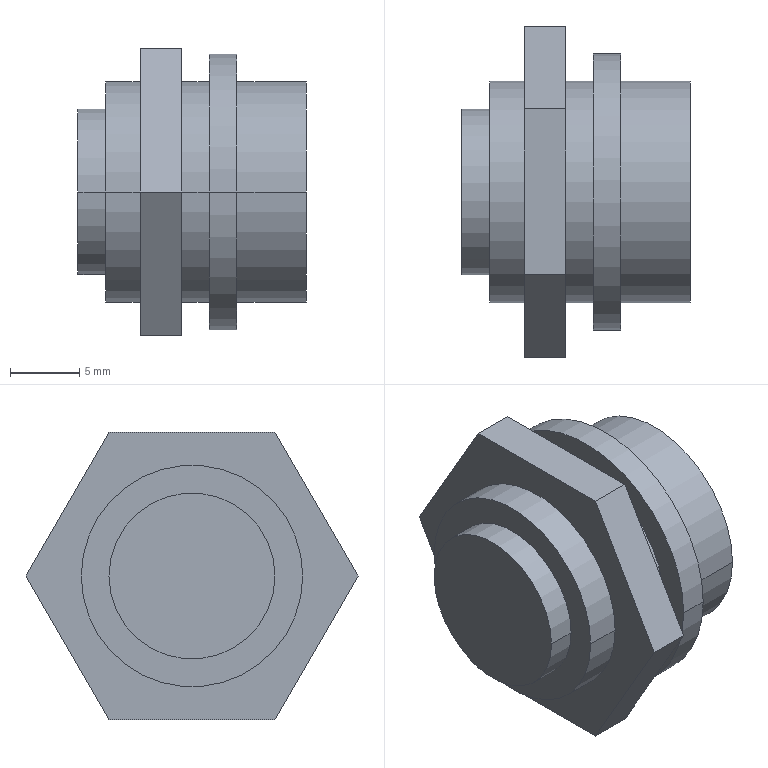Part | STEP file | Aviation connector M16-8AB | 1 solid | 23 faces | box 16.5 x 24 x 20.785 mm | volume 3887 mm3 | plane 13 | cylinder 10 | commonest cylinder face diameters 16 x6 12 x2 20 x2
STEP:
#1=CARTESIAN_POINT('',(0.,0.,0.));
#2=DIRECTION('',(0.,0.,1.));
#3=DIRECTION('',(1.,0.,0.));
#4=AXIS2_PLACEMENT_3D('',#1,#2,#3);
#5=CARTESIAN_POINT('',(11.5,8.,0.));
#6=VERTEX_POINT('',#5);
#7=CARTESIAN_POINT('',(11.5,-8.,0.));
#8=VERTEX_POINT('',#7);
#9=CARTESIAN_POINT('',(11.5,0.,0.));
#10=DIRECTION('',(1.,0.,0.));
#11=DIRECTION('',(0.,1.,0.));
#12=AXIS2_PLACEMENT_3D('',#9,#10,#11);
#13=CIRCLE('',#12,8.);
#14=CARTESIAN_POINT('',(16.5,0.,0.));
#15=DIRECTION('',(1.,0.,0.));
#16=DIRECTION('',(0.,1.,0.));
#17=AXIS2_PLACEMENT_3D('',#14,#15,#16);
#18=CYLINDRICAL_SURFACE('',#17,8.);
#19=CARTESIAN_POINT('',(0.,-5.));
#20=DIRECTION('',(1.,0.));
#21=VECTOR('',#20,1.);
#22=LINE('',#19,#21);
#23=(GEOMETRIC_REPRESENTATION_CONTEXT(2)PARAMETRIC_REPRESENTATION_CONTEXT()REPRESENTATION_CONTEXT('',''));
#24=DEFINITIONAL_REPRESENTATION('',(#22),#23);
#25=PCURVE('',#18,#24);
#26=CARTESIAN_POINT('',(11.5,10.,0.));
#27=DIRECTION('',(1.,0.,0.));
#28=DIRECTION('',(0.,1.,0.));
#29=AXIS2_PLACEMENT_3D('',#26,#27,#28);
#30=PLANE('',#29);
#31=CARTESIAN_POINT('',(-10.,0.));
#32=DIRECTION('',(1.,0.));
#33=AXIS2_PLACEMENT_2D('',#31,#32);
#34=CIRCLE('',#33,8.);
#35=(GEOMETRIC_REPRESENTATION_CONTEXT(2)PARAMETRIC_REPRESENTATION_CONTEXT()REPRESENTATION_CONTEXT('',''));
#36=DEFINITIONAL_REPRESENTATION('',(#34),#35);
#37=PCURVE('',#30,#36);
#38=SURFACE_CURVE('',#13,(#25,#37),.PCURVE_S1.);
#39=EDGE_CURVE('',#6,#8,#38,.T.);
#40=ORIENTED_EDGE('',*,*,#39,.T.);
#41=CARTESIAN_POINT('',(16.5,-8.,0.));
#42=VERTEX_POINT('',#41);
#43=CARTESIAN_POINT('',(16.5,-8.,0.));
#44=DIRECTION('',(1.,0.,0.));
#45=VECTOR('',#44,1.);
#46=LINE('',#43,#45);
#47=CARTESIAN_POINT('',(3.142,0.));
#48=DIRECTION('',(0.,1.));
#49=VECTOR('',#48,1.);
#50=LINE('',#47,#49);
#51=(GEOMETRIC_REPRESENTATION_CONTEXT(2)PARAMETRIC_REPRESENTATION_CONTEXT()REPRESENTATION_CONTEXT('',''));
#52=DEFINITIONAL_REPRESENTATION('',(#50),#51);
#53=PCURVE('',#18,#52);
#54=CARTESIAN_POINT('',(16.5,0.,0.));
#55=DIRECTION('',(1.,0.,0.));
#56=DIRECTION('',(0.,1.,0.));
#57=AXIS2_PLACEMENT_3D('',#54,#55,#56);
#58=CYLINDRICAL_SURFACE('',#57,8.);
#59=CARTESIAN_POINT('',(3.142,0.));
#60=DIRECTION('',(0.,1.));
#61=VECTOR('',#60,1.);
#62=LINE('',#59,#61);
#63=(GEOMETRIC_REPRESENTATION_CONTEXT(2)PARAMETRIC_REPRESENTATION_CONTEXT()REPRESENTATION_CONTEXT('',''));
#64=DEFINITIONAL_REPRESENTATION('',(#62),#63);
#65=PCURVE('',#58,#64);
#66=SURFACE_CURVE('',#46,(#53,#65),.PCURVE_S1.);
#67=EDGE_CURVE('',#8,#42,#66,.T.);
#68=ORIENTED_EDGE('',*,*,#67,.T.);
#69=CARTESIAN_POINT('',(16.5,8.,0.));
#70=VERTEX_POINT('',#69);
#71=CARTESIAN_POINT('',(16.5,0.,0.));
#72=DIRECTION('',(1.,0.,0.));
#73=DIRECTION('',(0.,1.,0.));
#74=AXIS2_PLACEMENT_3D('',#71,#72,#73);
#75=CIRCLE('',#74,8.);
#76=CARTESIAN_POINT('',(0.,0.));
#77=DIRECTION('',(1.,0.));
#78=VECTOR('',#77,1.);
#79=LINE('',#76,#78);
#80=(GEOMETRIC_REPRESENTATION_CONTEXT(2)PARAMETRIC_REPRESENTATION_CONTEXT()REPRESENTATION_CONTEXT('',''));
#81=DEFINITIONAL_REPRESENTATION('',(#79),#80);
#82=PCURVE('',#18,#81);
#83=CARTESIAN_POINT('',(16.5,8.,0.));
#84=DIRECTION('',(1.,0.,0.));
#85=DIRECTION('',(0.,1.,0.));
#86=AXIS2_PLACEMENT_3D('',#83,#84,#85);
#87=PLANE('',#86);
#88=CARTESIAN_POINT('',(-8.,0.));
#89=DIRECTION('',(1.,0.));
#90=AXIS2_PLACEMENT_2D('',#88,#89);
#91=CIRCLE('',#90,8.);
#92=(GEOMETRIC_REPRESENTATION_CONTEXT(2)PARAMETRIC_REPRESENTATION_CONTEXT()REPRESENTATION_CONTEXT('',''));
#93=DEFINITIONAL_REPRESENTATION('',(#91),#92);
#94=PCURVE('',#87,#93);
#95=SURFACE_CURVE('',#75,(#82,#94),.PCURVE_S1.);
#96=EDGE_CURVE('',#70,#42,#95,.T.);
#97=ORIENTED_EDGE('',*,*,#96,.F.);
#98=CARTESIAN_POINT('',(16.5,8.,0.));
#99=DIRECTION('',(1.,0.,0.));
#100=VECTOR('',#99,1.);
#101=LINE('',#98,#100);
#102=CARTESIAN_POINT('',(0.,0.));
#103=DIRECTION('',(0.,1.));
#104=VECTOR('',#103,1.);
#105=LINE('',#102,#104);
#106=(GEOMETRIC_REPRESENTATION_CONTEXT(2)PARAMETRIC_REPRESENTATION_CONTEXT()REPRESENTATION_CONTEXT('',''));
#107=DEFINITIONAL_REPRESENTATION('',(#105),#106);
#108=PCURVE('',#18,#107);
#109=CARTESIAN_POINT('',(6.283,0.));
#110=DIRECTION('',(0.,1.));
#111=VECTOR('',#110,1.);
#112=LINE('',#109,#111);
#113=(GEOMETRIC_REPRESENTATION_CONTEXT(2)PARAMETRIC_REPRESENTATION_CONTEXT()REPRESENTATION_CONTEXT('',''));
#114=DEFINITIONAL_REPRESENTATION('',(#112),#113);
#115=PCURVE('',#58,#114);
#116=SURFACE_CURVE('',#101,(#108,#115),.PCURVE_S1.);
#117=EDGE_CURVE('',#6,#70,#116,.T.);
#118=ORIENTED_EDGE('',*,*,#117,.F.);
#119=EDGE_LOOP('',(#40,#68,#97,#118));
#120=FACE_BOUND('',#119,.T.);
#121=ADVANCED_FACE('',(#120),#18,.T.);
#122=CARTESIAN_POINT('',(9.5,10.,0.));
#123=VERTEX_POINT('',#122);
#124=CARTESIAN_POINT('',(9.5,-10.,0.));
#125=VERTEX_POINT('',#124);
#126=CARTESIAN_POINT('',(9.5,0.,0.));
#127=DIRECTION('',(1.,0.,0.));
#128=DIRECTION('',(0.,1.,0.));
#129=AXIS2_PLACEMENT_3D('',#126,#127,#128);
#130=CIRCLE('',#129,10.);
#131=CARTESIAN_POINT('',(16.5,0.,0.));
#132=DIRECTION('',(1.,0.,0.));
#133=DIRECTION('',(0.,1.,0.));
#134=AXIS2_PLACEMENT_3D('',#131,#132,#133);
#135=CYLINDRICAL_SURFACE('',#134,10.);
#136=CARTESIAN_POINT('',(0.,-7.));
#137=DIRECTION('',(1.,0.));
#138=VECTOR('',#137,1.);
#139=LINE('',#136,#138);
#140=(GEOMETRIC_REPRESENTATION_CONTEXT(2)PARAMETRIC_REPRESENTATION_CONTEXT()REPRESENTATION_CONTEXT('',''));
#141=DEFINITIONAL_REPRESENTATION('',(#139),#140);
#142=PCURVE('',#135,#141);
#143=CARTESIAN_POINT('',(9.5,8.,0.));
#144=DIRECTION('',(-1.,0.,0.));
#145=DIRECTION('',(0.,-1.,0.));
#146=AXIS2_PLACEMENT_3D('',#143,#144,#145);
#147=PLANE('',#146);
#148=CARTESIAN_POINT('',(-2.,0.));
#149=CARTESIAN_POINT('',(-2.,17.321));
#150=CARTESIAN_POINT('',(13.,8.66));
#151=CARTESIAN_POINT('',(28.,0.));
#152=CARTESIAN_POINT('',(13.,-8.66));
#153=CARTESIAN_POINT('',(-2.,-17.321));
#154=CARTESIAN_POINT('',(-2.,0.));
#155=(BOUNDED_CURVE()B_SPLINE_CURVE(2,(#148,#149,#150,#151,#152,#153,#154),.UNSPECIFIED.,.T.,.F.)B_SPLINE_CURVE_WITH_KNOTS((1,2,2,2,2,1),(-2.094,0.,2.094,4.189,6.283,8.378),.UNSPECIFIED.)CURVE()GEOMETRIC_REPRESENTATION_ITEM()RATIONAL_B_SPLINE_CURVE((1.,0.5,1.,0.5,1.,0.5,1.))REPRESENTATION_ITEM(''));
#156=(GEOMETRIC_REPRESENTATION_CONTEXT(2)PARAMETRIC_REPRESENTATION_CONTEXT()REPRESENTATION_CONTEXT('',''));
#157=DEFINITIONAL_REPRESENTATION('',(#155),#156);
#158=PCURVE('',#147,#157);
#159=SURFACE_CURVE('',#130,(#142,#158),.PCURVE_S1.);
#160=EDGE_CURVE('',#123,#125,#159,.T.);
#161=ORIENTED_EDGE('',*,*,#160,.T.);
#162=CARTESIAN_POINT('',(11.5,-10.,0.));
#163=VERTEX_POINT('',#162);
#164=CARTESIAN_POINT('',(16.5,-10.,0.));
#165=DIRECTION('',(1.,0.,0.));
#166=VECTOR('',#165,1.);
#167=LINE('',#164,#166);
#168=CARTESIAN_POINT('',(3.142,0.));
#169=DIRECTION('',(0.,1.));
#170=VECTOR('',#169,1.);
#171=LINE('',#168,#170);
#172=(GEOMETRIC_REPRESENTATION_CONTEXT(2)PARAMETRIC_REPRESENTATION_CONTEXT()REPRESENTATION_CONTEXT('',''));
#173=DEFINITIONAL_REPRESENTATION('',(#171),#172);
#174=PCURVE('',#135,#173);
#175=CARTESIAN_POINT('',(16.5,0.,0.));
#176=DIRECTION('',(1.,0.,0.));
#177=DIRECTION('',(0.,1.,0.));
#178=AXIS2_PLACEMENT_3D('',#175,#176,#177);
#179=CYLINDRICAL_SURFACE('',#178,10.);
#180=CARTESIAN_POINT('',(3.142,0.));
#181=DIRECTION('',(0.,1.));
#182=VECTOR('',#181,1.);
#183=LINE('',#180,#182);
#184=(GEOMETRIC_REPRESENTATION_CONTEXT(2)PARAMETRIC_REPRESENTATION_CONTEXT()REPRESENTATION_CONTEXT('',''));
#185=DEFINITIONAL_REPRESENTATION('',(#183),#184);
#186=PCURVE('',#179,#185);
#187=SURFACE_CURVE('',#167,(#174,#186),.PCURVE_S1.);
#188=EDGE_CURVE('',#125,#163,#187,.T.);
#189=ORIENTED_EDGE('',*,*,#188,.T.);
#190=CARTESIAN_POINT('',(11.5,10.,0.));
#191=VERTEX_POINT('',#190);
#192=CARTESIAN_POINT('',(11.5,0.,0.));
#193=DIRECTION('',(1.,0.,0.));
#194=DIRECTION('',(0.,1.,0.));
#195=AXIS2_PLACEMENT_3D('',#192,#193,#194);
#196=CIRCLE('',#195,10.);
#197=CARTESIAN_POINT('',(0.,-5.));
#198=DIRECTION('',(1.,0.));
#199=VECTOR('',#198,1.);
#200=LINE('',#197,#199);
#201=(GEOMETRIC_REPRESENTATION_CONTEXT(2)PARAMETRIC_REPRESENTATION_CONTEXT()REPRESENTATION_CONTEXT('',''));
#202=DEFINITIONAL_REPRESENTATION('',(#200),#201);
#203=PCURVE('',#135,#202);
#204=CARTESIAN_POINT('',(-10.,0.));
#205=DIRECTION('',(1.,0.));
#206=AXIS2_PLACEMENT_2D('',#204,#205);
#207=CIRCLE('',#206,10.);
#208=(GEOMETRIC_REPRESENTATION_CONTEXT(2)PARAMETRIC_REPRESENTATION_CONTEXT()REPRESENTATION_CONTEXT('',''));
#209=DEFINITIONAL_REPRESENTATION('',(#207),#208);
#210=PCURVE('',#30,#209);
#211=SURFACE_CURVE('',#196,(#203,#210),.PCURVE_S1.);
#212=EDGE_CURVE('',#191,#163,#211,.T.);
#213=ORIENTED_EDGE('',*,*,#212,.F.);
#214=CARTESIAN_POINT('',(16.5,10.,0.));
#215=DIRECTION('',(1.,0.,0.));
#216=VECTOR('',#215,1.);
#217=LINE('',#214,#216);
#218=CARTESIAN_POINT('',(0.,0.));
#219=DIRECTION('',(0.,1.));
#220=VECTOR('',#219,1.);
#221=LINE('',#218,#220);
#222=(GEOMETRIC_REPRESENTATION_CONTEXT(2)PARAMETRIC_REPRESENTATION_CONTEXT()REPRESENTATION_CONTEXT('',''));
#223=DEFINITIONAL_REPRESENTATION('',(#221),#222);
#224=PCURVE('',#135,#223);
#225=CARTESIAN_POINT('',(6.283,0.));
#226=DIRECTION('',(0.,1.));
#227=VECTOR('',#226,1.);
#228=LINE('',#225,#227);
#229=(GEOMETRIC_REPRESENTATION_CONTEXT(2)PARAMETRIC_REPRESENTATION_CONTEXT()REPRESENTATION_CONTEXT('',''));
#230=DEFINITIONAL_REPRESENTATION('',(#228),#229);
#231=PCURVE('',#179,#230);
#232=SURFACE_CURVE('',#217,(#224,#231),.PCURVE_S1.);
#233=EDGE_CURVE('',#123,#191,#232,.T.);
#234=ORIENTED_EDGE('',*,*,#233,.F.);
#235=EDGE_LOOP('',(#161,#189,#213,#234));
#236=FACE_BOUND('',#235,.T.);
#237=ADVANCED_FACE('',(#236),#135,.T.);
#238=CARTESIAN_POINT('',(7.5,8.,0.));
#239=VERTEX_POINT('',#238);
#240=CARTESIAN_POINT('',(7.5,-8.,0.));
#241=VERTEX_POINT('',#240);
#242=CARTESIAN_POINT('',(7.5,0.,0.));
#243=DIRECTION('',(1.,0.,0.));
#244=DIRECTION('',(0.,1.,0.));
#245=AXIS2_PLACEMENT_3D('',#242,#243,#244);
#246=CIRCLE('',#245,8.);
#247=CARTESIAN_POINT('',(16.5,0.,0.));
#248=DIRECTION('',(1.,0.,0.));
#249=DIRECTION('',(0.,1.,0.));
#250=AXIS2_PLACEMENT_3D('',#247,#248,#249);
#251=CYLINDRICAL_SURFACE('',#250,8.);
#252=CARTESIAN_POINT('',(0.,-9.));
#253=DIRECTION('',(1.,0.));
#254=VECTOR('',#253,1.);
#255=LINE('',#252,#254);
#256=(GEOMETRIC_REPRESENTATION_CONTEXT(2)PARAMETRIC_REPRESENTATION_CONTEXT()REPRESENTATION_CONTEXT('',''));
#257=DEFINITIONAL_REPRESENTATION('',(#255),#256);
#258=PCURVE('',#251,#257);
#259=CARTESIAN_POINT('',(7.5,12.,0.));
#260=DIRECTION('',(1.,0.,0.));
#261=DIRECTION('',(0.,1.,0.));
#262=AXIS2_PLACEMENT_3D('',#259,#260,#261);
#263=PLANE('',#262);
#264=CARTESIAN_POINT('',(-12.,0.));
#265=DIRECTION('',(1.,0.));
#266=AXIS2_PLACEMENT_2D('',#264,#265);
#267=CIRCLE('',#266,8.);
#268=(GEOMETRIC_REPRESENTATION_CONTEXT(2)PARAMETRIC_REPRESENTATION_CONTEXT()REPRESENTATION_CONTEXT('',''));
#269=DEFINITIONAL_REPRESENTATION('',(#267),#268);
#270=PCURVE('',#263,#269);
#271=SURFACE_CURVE('',#246,(#258,#270),.PCURVE_S1.);
#272=EDGE_CURVE('',#239,#241,#271,.T.);
#273=ORIENTED_EDGE('',*,*,#272,.T.);
#274=CARTESIAN_POINT('',(9.5,-8.,0.));
#275=VERTEX_POINT('',#274);
#276=CARTESIAN_POINT('',(16.5,-8.,0.));
#277=DIRECTION('',(1.,0.,0.));
#278=VECTOR('',#277,1.);
#279=LINE('',#276,#278);
#280=CARTESIAN_POINT('',(3.142,0.));
#281=DIRECTION('',(0.,1.));
#282=VECTOR('',#281,1.);
#283=LINE('',#280,#282);
#284=(GEOMETRIC_REPRESENTATION_CONTEXT(2)PARAMETRIC_REPRESENTATION_CONTEXT()REPRESENTATION_CONTEXT('',''));
#285=DEFINITIONAL_REPRESENTATION('',(#283),#284);
#286=PCURVE('',#251,#285);
#287=CARTESIAN_POINT('',(16.5,0.,0.));
#288=DIRECTION('',(1.,0.,0.));
#289=DIRECTION('',(0.,1.,0.));
#290=AXIS2_PLACEMENT_3D('',#287,#288,#289);
#291=CYLINDRICAL_SURFACE('',#290,8.);
#292=CARTESIAN_POINT('',(3.142,0.));
#293=DIRECTION('',(0.,1.));
#294=VECTOR('',#293,1.);
#295=LINE('',#292,#294);
#296=(GEOMETRIC_REPRESENTATION_CONTEXT(2)PARAMETRIC_REPRESENTATION_CONTEXT()REPRESENTATION_CONTEXT('',''));
#297=DEFINITIONAL_REPRESENTATION('',(#295),#296);
#298=PCURVE('',#291,#297);
#299=SURFACE_CURVE('',#279,(#286,#298),.PCURVE_S1.);
#300=EDGE_CURVE('',#241,#275,#299,.T.);
#301=ORIENTED_EDGE('',*,*,#300,.T.);
#302=CARTESIAN_POINT('',(9.5,8.,0.));
#303=VERTEX_POINT('',#302);
#304=CARTESIAN_POINT('',(9.5,0.,0.));
#305=DIRECTION('',(1.,0.,0.));
#306=DIRECTION('',(0.,1.,0.));
#307=AXIS2_PLACEMENT_3D('',#304,#305,#306);
#308=CIRCLE('',#307,8.);
#309=CARTESIAN_POINT('',(0.,-7.));
#310=DIRECTION('',(1.,0.));
#311=VECTOR('',#310,1.);
#312=LINE('',#309,#311);
#313=(GEOMETRIC_REPRESENTATION_CONTEXT(2)PARAMETRIC_REPRESENTATION_CONTEXT()REPRESENTATION_CONTEXT('',''));
#314=DEFINITIONAL_REPRESENTATION('',(#312),#313);
#315=PCURVE('',#251,#314);
#316=CARTESIAN_POINT('',(0.,0.));
#317=CARTESIAN_POINT('',(0.,13.856));
#318=CARTESIAN_POINT('',(12.,6.928));
#319=CARTESIAN_POINT('',(24.,0.));
#320=CARTESIAN_POINT('',(12.,-6.928));
#321=CARTESIAN_POINT('',(0.,-13.856));
#322=CARTESIAN_POINT('',(0.,0.));
#323=(BOUNDED_CURVE()B_SPLINE_CURVE(2,(#316,#317,#318,#319,#320,#321,#322),.UNSPECIFIED.,.T.,.F.)B_SPLINE_CURVE_WITH_KNOTS((1,2,2,2,2,1),(-2.094,0.,2.094,4.189,6.283,8.378),.UNSPECIFIED.)CURVE()GEOMETRIC_REPRESENTATION_ITEM()RATIONAL_B_SPLINE_CURVE((1.,0.5,1.,0.5,1.,0.5,1.))REPRESENTATION_ITEM(''));
#324=(GEOMETRIC_REPRESENTATION_CONTEXT(2)PARAMETRIC_REPRESENTATION_CONTEXT()REPRESENTATION_CONTEXT('',''));
#325=DEFINITIONAL_REPRESENTATION('',(#323),#324);
#326=PCURVE('',#147,#325);
#327=SURFACE_CURVE('',#308,(#315,#326),.PCURVE_S1.);
#328=EDGE_CURVE('',#303,#275,#327,.T.);
#329=ORIENTED_EDGE('',*,*,#328,.F.);
#330=CARTESIAN_POINT('',(16.5,8.,0.));
#331=DIRECTION('',(1.,0.,0.));
#332=VECTOR('',#331,1.);
#333=LINE('',#330,#332);
#334=CARTESIAN_POINT('',(0.,0.));
#335=DIRECTION('',(0.,1.));
#336=VECTOR('',#335,1.);
#337=LINE('',#334,#336);
#338=(GEOMETRIC_REPRESENTATION_CONTEXT(2)PARAMETRIC_REPRESENTATION_CONTEXT()REPRESENTATION_CONTEXT('',''));
#339=DEFINITIONAL_REPRESENTATION('',(#337),#338);
#340=PCURVE('',#251,#339);
#341=CARTESIAN_POINT('',(6.283,0.));
#342=DIRECTION('',(0.,1.));
#343=VECTOR('',#342,1.);
#344=LINE('',#341,#343);
#345=(GEOMETRIC_REPRESENTATION_CONTEXT(2)PARAMETRIC_REPRESENTATION_CONTEXT()REPRESENTATION_CONTEXT('',''));
#346=DEFINITIONAL_REPRESENTATION('',(#344),#345);
#347=PCURVE('',#291,#346);
#348=SURFACE_CURVE('',#333,(#340,#347),.PCURVE_S1.);
#349=EDGE_CURVE('',#239,#303,#348,.T.);
#350=ORIENTED_EDGE('',*,*,#349,.F.);
#351=EDGE_LOOP('',(#273,#301,#329,#350));
#352=FACE_BOUND('',#351,.T.);
#353=ADVANCED_FACE('',(#352),#251,.T.);
#354=CARTESIAN_POINT('',(2.,8.,0.));
#355=VERTEX_POINT('',#354);
#356=CARTESIAN_POINT('',(2.,-8.,0.));
#357=VERTEX_POINT('',#356);
#358=CARTESIAN_POINT('',(2.,0.,0.));
#359=DIRECTION('',(1.,0.,0.));
#360=DIRECTION('',(0.,1.,0.));
#361=AXIS2_PLACEMENT_3D('',#358,#359,#360);
#362=CIRCLE('',#361,8.);
#363=CARTESIAN_POINT('',(16.5,0.,0.));
#364=DIRECTION('',(1.,0.,0.));
#365=DIRECTION('',(0.,1.,0.));
#366=AXIS2_PLACEMENT_3D('',#363,#364,#365);
#367=CYLINDRICAL_SURFACE('',#366,8.);
#368=CARTESIAN_POINT('',(0.,-14.5));
#369=DIRECTION('',(1.,0.));
#370=VECTOR('',#369,1.);
#371=LINE('',#368,#370);
#372=(GEOMETRIC_REPRESENTATION_CONTEXT(2)PARAMETRIC_REPRESENTATION_CONTEXT()REPRESENTATION_CONTEXT('',''));
#373=DEFINITIONAL_REPRESENTATION('',(#371),#372);
#374=PCURVE('',#367,#373);
#375=CARTESIAN_POINT('',(2.,6.,0.));
#376=DIRECTION('',(-1.,0.,0.));
#377=DIRECTION('',(0.,-1.,0.));
#378=AXIS2_PLACEMENT_3D('',#375,#376,#377);
#379=PLANE('',#378);
#380=CARTESIAN_POINT('',(-2.,0.));
#381=CARTESIAN_POINT('',(-2.,13.856));
#382=CARTESIAN_POINT('',(10.,6.928));
#383=CARTESIAN_POINT('',(22.,0.));
#384=CARTESIAN_POINT('',(10.,-6.928));
#385=CARTESIAN_POINT('',(-2.,-13.856));
#386=CARTESIAN_POINT('',(-2.,0.));
#387=(BOUNDED_CURVE()B_SPLINE_CURVE(2,(#380,#381,#382,#383,#384,#385,#386),.UNSPECIFIED.,.T.,.F.)B_SPLINE_CURVE_WITH_KNOTS((1,2,2,2,2,1),(-2.094,0.,2.094,4.189,6.283,8.378),.UNSPECIFIED.)CURVE()GEOMETRIC_REPRESENTATION_ITEM()RATIONAL_B_SPLINE_CURVE((1.,0.5,1.,0.5,1.,0.5,1.))REPRESENTATION_ITEM(''));
#388=(GEOMETRIC_REPRESENTATION_CONTEXT(2)PARAMETRIC_REPRESENTATION_CONTEXT()REPRESENTATION_CONTEXT('',''));
#389=DEFINITIONAL_REPRESENTATION('',(#387),#388);
#390=PCURVE('',#379,#389);
#391=SURFACE_CURVE('',#362,(#374,#390),.PCURVE_S1.);
#392=EDGE_CURVE('',#355,#357,#391,.T.);
#393=ORIENTED_EDGE('',*,*,#392,.T.);
#394=CARTESIAN_POINT('',(4.5,-8.,0.));
#395=VERTEX_POINT('',#394);
#396=CARTESIAN_POINT('',(16.5,-8.,0.));
#397=DIRECTION('',(1.,0.,0.));
#398=VECTOR('',#397,1.);
#399=LINE('',#396,#398);
#400=CARTESIAN_POINT('',(3.142,0.));
#401=DIRECTION('',(0.,1.));
#402=VECTOR('',#401,1.);
#403=LINE('',#400,#402);
#404=(GEOMETRIC_REPRESENTATION_CONTEXT(2)PARAMETRIC_REPRESENTATION_CONTEXT()REPRESENTATION_CONTEXT('',''));
#405=DEFINITIONAL_REPRESENTATION('',(#403),#404);
#406=PCURVE('',#367,#405);
#407=CARTESIAN_POINT('',(16.5,0.,0.));
#408=DIRECTION('',(1.,0.,0.));
#409=DIRECTION('',(0.,1.,0.));
#410=AXIS2_PLACEMENT_3D('',#407,#408,#409);
#411=CYLINDRICAL_SURFACE('',#410,8.);
#412=CARTESIAN_POINT('',(3.142,0.));
#413=DIRECTION('',(0.,1.));
#414=VECTOR('',#413,1.);
#415=LINE('',#412,#414);
#416=(GEOMETRIC_REPRESENTATION_CONTEXT(2)PARAMETRIC_REPRESENTATION_CONTEXT()REPRESENTATION_CONTEXT('',''));
#417=DEFINITIONAL_REPRESENTATION('',(#415),#416);
#418=PCURVE('',#411,#417);
#419=SURFACE_CURVE('',#399,(#406,#418),.PCURVE_S1.);
#420=EDGE_CURVE('',#357,#395,#419,.T.);
#421=ORIENTED_EDGE('',*,*,#420,.T.);
#422=CARTESIAN_POINT('',(4.5,8.,0.));
#423=VERTEX_POINT('',#422);
#424=CARTESIAN_POINT('',(4.5,0.,0.));
#425=DIRECTION('',(1.,0.,0.));
#426=DIRECTION('',(0.,1.,0.));
#427=AXIS2_PLACEMENT_3D('',#424,#425,#426);
#428=CIRCLE('',#427,8.);
#429=CARTESIAN_POINT('',(0.,-12.));
#430=DIRECTION('',(1.,0.));
#431=VECTOR('',#430,1.);
#432=LINE('',#429,#431);
#433=(GEOMETRIC_REPRESENTATION_CONTEXT(2)PARAMETRIC_REPRESENTATION_CONTEXT()REPRESENTATION_CONTEXT('',''));
#434=DEFINITIONAL_REPRESENTATION('',(#432),#433);
#435=PCURVE('',#367,#434);
#436=CARTESIAN_POINT('',(4.5,8.,0.));
#437=DIRECTION('',(-1.,0.,0.));
#438=DIRECTION('',(0.,-1.,0.));
#439=AXIS2_PLACEMENT_3D('',#436,#437,#438);
#440=PLANE('',#439);
#441=CARTESIAN_POINT('',(0.,0.));
#442=CARTESIAN_POINT('',(0.,13.856));
#443=CARTESIAN_POINT('',(12.,6.928));
#444=CARTESIAN_POINT('',(24.,0.));
#445=CARTESIAN_POINT('',(12.,-6.928));
#446=CARTESIAN_POINT('',(0.,-13.856));
#447=CARTESIAN_POINT('',(0.,0.));
#448=(BOUNDED_CURVE()B_SPLINE_CURVE(2,(#441,#442,#443,#444,#445,#446,#447),.UNSPECIFIED.,.T.,.F.)B_SPLINE_CURVE_WITH_KNOTS((1,2,2,2,2,1),(-2.094,0.,2.094,4.189,6.283,8.378),.UNSPECIFIED.)CURVE()GEOMETRIC_REPRESENTATION_ITEM()RATIONAL_B_SPLINE_CURVE((1.,0.5,1.,0.5,1.,0.5,1.))REPRESENTATION_ITEM(''));
#449=(GEOMETRIC_REPRESENTATION_CONTEXT(2)PARAMETRIC_REPRESENTATION_CONTEXT()REPRESENTATION_CONTEXT('',''));
#450=DEFINITIONAL_REPRESENTATION('',(#448),#449);
#451=PCURVE('',#440,#450);
#452=SURFACE_CURVE('',#428,(#435,#451),.PCURVE_S1.);
#453=EDGE_CURVE('',#423,#395,#452,.T.);
#454=ORIENTED_EDGE('',*,*,#453,.F.);
#455=CARTESIAN_POINT('',(16.5,8.,0.));
#456=DIRECTION('',(1.,0.,0.));
#457=VECTOR('',#456,1.);
#458=LINE('',#455,#457);
#459=CARTESIAN_POINT('',(0.,0.));
#460=DIRECTION('',(0.,1.));
#461=VECTOR('',#460,1.);
#462=LINE('',#459,#461);
#463=(GEOMETRIC_REPRESENTATION_CONTEXT(2)PARAMETRIC_REPRESENTATION_CONTEXT()REPRESENTATION_CONTEXT('',''));
#464=DEFINITIONAL_REPRESENTATION('',(#462),#463);
#465=PCURVE('',#367,#464);
#466=CARTESIAN_POINT('',(6.283,0.));
#467=DIRECTION('',(0.,1.));
#468=VECTOR('',#467,1.);
#469=LINE('',#466,#468);
#470=(GEOMETRIC_REPRESENTATION_CONTEXT(2)PARAMETRIC_REPRESENTATION_CONTEXT()REPRESENTATION_CONTEXT('',''));
#471=DEFINITIONAL_REPRESENTATION('',(#469),#470);
#472=PCURVE('',#411,#471);
#473=SURFACE_CURVE('',#458,(#465,#472),.PCURVE_S1.);
#474=EDGE_CURVE('',#355,#423,#473,.T.);
#475=ORIENTED_EDGE('',*,*,#474,.F.);
#476=EDGE_LOOP('',(#393,#421,#454,#475));
#477=FACE_BOUND('',#476,.T.);
#478=ADVANCED_FACE('',(#477),#367,.T.);
#479=CARTESIAN_POINT('',(0.,6.,0.));
#480=VERTEX_POINT('',#479);
#481=CARTESIAN_POINT('',(0.,-6.,0.));
#482=VERTEX_POINT('',#481);
#483=CARTESIAN_POINT('',(0.,0.,0.));
#484=DIRECTION('',(1.,0.,0.));
#485=DIRECTION('',(0.,1.,0.));
#486=AXIS2_PLACEMENT_3D('',#483,#484,#485);
#487=CIRCLE('',#486,6.);
#488=CARTESIAN_POINT('',(16.5,0.,0.));
#489=DIRECTION('',(1.,0.,0.));
#490=DIRECTION('',(0.,1.,0.));
#491=AXIS2_PLACEMENT_3D('',#488,#489,#490);
#492=CYLINDRICAL_SURFACE('',#491,6.);
#493=CARTESIAN_POINT('',(0.,-16.5));
#494=DIRECTION('',(1.,0.));
#495=VECTOR('',#494,1.);
#496=LINE('',#493,#495);
#497=(GEOMETRIC_REPRESENTATION_CONTEXT(2)PARAMETRIC_REPRESENTATION_CONTEXT()REPRESENTATION_CONTEXT('',''));
#498=DEFINITIONAL_REPRESENTATION('',(#496),#497);
#499=PCURVE('',#492,#498);
#500=CARTESIAN_POINT('',(0.,0.,0.));
#501=DIRECTION('',(-1.,0.,0.));
#502=DIRECTION('',(0.,-1.,0.));
#503=AXIS2_PLACEMENT_3D('',#500,#501,#502);
#504=PLANE('',#503);
#505=CARTESIAN_POINT('',(-6.,0.));
#506=CARTESIAN_POINT('',(-6.,10.392));
#507=CARTESIAN_POINT('',(3.,5.196));
#508=CARTESIAN_POINT('',(12.,0.));
#509=CARTESIAN_POINT('',(3.,-5.196));
#510=CARTESIAN_POINT('',(-6.,-10.392));
#511=CARTESIAN_POINT('',(-6.,0.));
#512=(BOUNDED_CURVE()B_SPLINE_CURVE(2,(#505,#506,#507,#508,#509,#510,#511),.UNSPECIFIED.,.T.,.F.)B_SPLINE_CURVE_WITH_KNOTS((1,2,2,2,2,1),(-2.094,0.,2.094,4.189,6.283,8.378),.UNSPECIFIED.)CURVE()GEOMETRIC_REPRESENTATION_ITEM()RATIONAL_B_SPLINE_CURVE((1.,0.5,1.,0.5,1.,0.5,1.))REPRESENTATION_ITEM(''));
#513=(GEOMETRIC_REPRESENTATION_CONTEXT(2)PARAMETRIC_REPRESENTATION_CONTEXT()REPRESENTATION_CONTEXT('',''));
#514=DEFINITIONAL_REPRESENTATION('',(#512),#513);
#515=PCURVE('',#504,#514);
#516=SURFACE_CURVE('',#487,(#499,#515),.PCURVE_S1.);
#517=EDGE_CURVE('',#480,#482,#516,.T.);
#518=ORIENTED_EDGE('',*,*,#517,.T.);
#519=CARTESIAN_POINT('',(2.,-6.,0.));
#520=VERTEX_POINT('',#519);
#521=CARTESIAN_POINT('',(16.5,-6.,0.));
#522=DIRECTION('',(1.,0.,0.));
#523=VECTOR('',#522,1.);
#524=LINE('',#521,#523);
#525=CARTESIAN_POINT('',(3.142,0.));
#526=DIRECTION('',(0.,1.));
#527=VECTOR('',#526,1.);
#528=LINE('',#525,#527);
#529=(GEOMETRIC_REPRESENTATION_CONTEXT(2)PARAMETRIC_REPRESENTATION_CONTEXT()REPRESENTATION_CONTEXT('',''));
#530=DEFINITIONAL_REPRESENTATION('',(#528),#529);
#531=PCURVE('',#492,#530);
#532=CARTESIAN_POINT('',(16.5,0.,0.));
#533=DIRECTION('',(1.,0.,0.));
#534=DIRECTION('',(0.,1.,0.));
#535=AXIS2_PLACEMENT_3D('',#532,#533,#534);
#536=CYLINDRICAL_SURFACE('',#535,6.);
#537=CARTESIAN_POINT('',(3.142,0.));
#538=DIRECTION('',(0.,1.));
#539=VECTOR('',#538,1.);
#540=LINE('',#537,#539);
#541=(GEOMETRIC_REPRESENTATION_CONTEXT(2)PARAMETRIC_REPRESENTATION_CONTEXT()REPRESENTATION_CONTEXT('',''));
#542=DEFINITIONAL_REPRESENTATION('',(#540),#541);
#543=PCURVE('',#536,#542);
#544=SURFACE_CURVE('',#524,(#531,#543),.PCURVE_S1.);
#545=EDGE_CURVE('',#482,#520,#544,.T.);
#546=ORIENTED_EDGE('',*,*,#545,.T.);
#547=CARTESIAN_POINT('',(2.,6.,0.));
#548=VERTEX_POINT('',#547);
#549=CARTESIAN_POINT('',(2.,0.,0.));
#550=DIRECTION('',(1.,0.,0.));
#551=DIRECTION('',(0.,1.,0.));
#552=AXIS2_PLACEMENT_3D('',#549,#550,#551);
#553=CIRCLE('',#552,6.);
#554=CARTESIAN_POINT('',(0.,-14.5));
#555=DIRECTION('',(1.,0.));
#556=VECTOR('',#555,1.);
#557=LINE('',#554,#556);
#558=(GEOMETRIC_REPRESENTATION_CONTEXT(2)PARAMETRIC_REPRESENTATION_CONTEXT()REPRESENTATION_CONTEXT('',''));
#559=DEFINITIONAL_REPRESENTATION('',(#557),#558);
#560=PCURVE('',#492,#559);
#561=CARTESIAN_POINT('',(0.,0.));
#562=CARTESIAN_POINT('',(0.,10.392));
#563=CARTESIAN_POINT('',(9.,5.196));
#564=CARTESIAN_POINT('',(18.,0.));
#565=CARTESIAN_POINT('',(9.,-5.196));
#566=CARTESIAN_POINT('',(0.,-10.392));
#567=CARTESIAN_POINT('',(0.,0.));
#568=(BOUNDED_CURVE()B_SPLINE_CURVE(2,(#561,#562,#563,#564,#565,#566,#567),.UNSPECIFIED.,.T.,.F.)B_SPLINE_CURVE_WITH_KNOTS((1,2,2,2,2,1),(-2.094,0.,2.094,4.189,6.283,8.378),.UNSPECIFIED.)CURVE()GEOMETRIC_REPRESENTATION_ITEM()RATIONAL_B_SPLINE_CURVE((1.,0.5,1.,0.5,1.,0.5,1.))REPRESENTATION_ITEM(''));
#569=(GEOMETRIC_REPRESENTATION_CONTEXT(2)PARAMETRIC_REPRESENTATION_CONTEXT()REPRESENTATION_CONTEXT('',''));
#570=DEFINITIONAL_REPRESENTATION('',(#568),#569);
#571=PCURVE('',#379,#570);
#572=SURFACE_CURVE('',#553,(#560,#571),.PCURVE_S1.);
#573=EDGE_CURVE('',#548,#520,#572,.T.);
#574=ORIENTED_EDGE('',*,*,#573,.F.);
#575=CARTESIAN_POINT('',(16.5,6.,0.));
#576=DIRECTION('',(1.,0.,0.));
#577=VECTOR('',#576,1.);
#578=LINE('',#575,#577);
#579=CARTESIAN_POINT('',(0.,0.));
#580=DIRECTION('',(0.,1.));
#581=VECTOR('',#580,1.);
#582=LINE('',#579,#581);
#583=(GEOMETRIC_REPRESENTATION_CONTEXT(2)PARAMETRIC_REPRESENTATION_CONTEXT()REPRESENTATION_CONTEXT('',''));
#584=DEFINITIONAL_REPRESENTATION('',(#582),#583);
#585=PCURVE('',#492,#584);
#586=CARTESIAN_POINT('',(6.283,0.));
#587=DIRECTION('',(0.,1.));
#588=VECTOR('',#587,1.);
#589=LINE('',#586,#588);
#590=(GEOMETRIC_REPRESENTATION_CONTEXT(2)PARAMETRIC_REPRESENTATION_CONTEXT()REPRESENTATION_CONTEXT('',''));
#591=DEFINITIONAL_REPRESENTATION('',(#589),#590);
#592=PCURVE('',#536,#591);
#593=SURFACE_CURVE('',#578,(#585,#592),.PCURVE_S1.);
#594=EDGE_CURVE('',#480,#548,#593,.T.);
#595=ORIENTED_EDGE('',*,*,#594,.F.);
#596=EDGE_LOOP('',(#518,#546,#574,#595));
#597=FACE_BOUND('',#596,.T.);
#598=ADVANCED_FACE('',(#597),#492,.T.);
#599=ORIENTED_EDGE('',*,*,#96,.T.);
#600=CARTESIAN_POINT('',(16.5,0.,0.));
#601=DIRECTION('',(1.,0.,0.));
#602=DIRECTION('',(0.,1.,0.));
#603=AXIS2_PLACEMENT_3D('',#600,#601,#602);
#604=CIRCLE('',#603,8.);
#605=CARTESIAN_POINT('',(-8.,0.));
#606=DIRECTION('',(1.,0.));
#607=AXIS2_PLACEMENT_2D('',#605,#606);
#608=CIRCLE('',#607,8.);
#609=(GEOMETRIC_REPRESENTATION_CONTEXT(2)PARAMETRIC_REPRESENTATION_CONTEXT()REPRESENTATION_CONTEXT('',''));
#610=DEFINITIONAL_REPRESENTATION('',(#608),#609);
#611=PCURVE('',#87,#610);
#612=CARTESIAN_POINT('',(0.,0.));
#613=DIRECTION('',(1.,0.));
#614=VECTOR('',#613,1.);
#615=LINE('',#612,#614);
#616=(GEOMETRIC_REPRESENTATION_CONTEXT(2)PARAMETRIC_REPRESENTATION_CONTEXT()REPRESENTATION_CONTEXT('',''));
#617=DEFINITIONAL_REPRESENTATION('',(#615),#616);
#618=PCURVE('',#58,#617);
#619=SURFACE_CURVE('',#604,(#611,#618),.PCURVE_S1.);
#620=EDGE_CURVE('',#42,#70,#619,.T.);
#621=ORIENTED_EDGE('',*,*,#620,.T.);
#622=EDGE_LOOP('',(#599,#621));
#623=FACE_BOUND('',#622,.T.);
#624=ADVANCED_FACE('',(#623),#87,.T.);
#625=ORIENTED_EDGE('',*,*,#67,.F.);
#626=CARTESIAN_POINT('',(11.5,0.,0.));
#627=DIRECTION('',(1.,0.,0.));
#628=DIRECTION('',(0.,1.,0.));
#629=AXIS2_PLACEMENT_3D('',#626,#627,#628);
#630=CIRCLE('',#629,8.);
#631=CARTESIAN_POINT('',(0.,-5.));
#632=DIRECTION('',(1.,0.));
#633=VECTOR('',#632,1.);
#634=LINE('',#631,#633);
#635=(GEOMETRIC_REPRESENTATION_CONTEXT(2)PARAMETRIC_REPRESENTATION_CONTEXT()REPRESENTATION_CONTEXT('',''));
#636=DEFINITIONAL_REPRESENTATION('',(#634),#635);
#637=PCURVE('',#58,#636);
#638=CARTESIAN_POINT('',(-10.,0.));
#639=DIRECTION('',(1.,0.));
#640=AXIS2_PLACEMENT_2D('',#638,#639);
#641=CIRCLE('',#640,8.);
#642=(GEOMETRIC_REPRESENTATION_CONTEXT(2)PARAMETRIC_REPRESENTATION_CONTEXT()REPRESENTATION_CONTEXT('',''));
#643=DEFINITIONAL_REPRESENTATION('',(#641),#642);
#644=PCURVE('',#30,#643);
#645=SURFACE_CURVE('',#630,(#637,#644),.PCURVE_S1.);
#646=EDGE_CURVE('',#8,#6,#645,.T.);
#647=ORIENTED_EDGE('',*,*,#646,.T.);
#648=ORIENTED_EDGE('',*,*,#117,.T.);
#649=ORIENTED_EDGE('',*,*,#620,.F.);
#650=EDGE_LOOP('',(#625,#647,#648,#649));
#651=FACE_BOUND('',#650,.T.);
#652=ADVANCED_FACE('',(#651),#58,.T.);
#653=ORIENTED_EDGE('',*,*,#39,.F.);
#654=ORIENTED_EDGE('',*,*,#646,.F.);
#655=EDGE_LOOP('',(#653,#654));
#656=FACE_BOUND('',#655,.T.);
#657=ORIENTED_EDGE('',*,*,#212,.T.);
#658=CARTESIAN_POINT('',(11.5,0.,0.));
#659=DIRECTION('',(1.,0.,0.));
#660=DIRECTION('',(0.,1.,0.));
#661=AXIS2_PLACEMENT_3D('',#658,#659,#660);
#662=CIRCLE('',#661,10.);
#663=CARTESIAN_POINT('',(-10.,0.));
#664=DIRECTION('',(1.,0.));
#665=AXIS2_PLACEMENT_2D('',#663,#664);
#666=CIRCLE('',#665,10.);
#667=(GEOMETRIC_REPRESENTATION_CONTEXT(2)PARAMETRIC_REPRESENTATION_CONTEXT()REPRESENTATION_CONTEXT('',''));
#668=DEFINITIONAL_REPRESENTATION('',(#666),#667);
#669=PCURVE('',#30,#668);
#670=CARTESIAN_POINT('',(0.,-5.));
#671=DIRECTION('',(1.,0.));
#672=VECTOR('',#671,1.);
#673=LINE('',#670,#672);
#674=(GEOMETRIC_REPRESENTATION_CONTEXT(2)PARAMETRIC_REPRESENTATION_CONTEXT()REPRESENTATION_CONTEXT('',''));
#675=DEFINITIONAL_REPRESENTATION('',(#673),#674);
#676=PCURVE('',#179,#675);
#677=SURFACE_CURVE('',#662,(#669,#676),.PCURVE_S1.);
#678=EDGE_CURVE('',#163,#191,#677,.T.);
#679=ORIENTED_EDGE('',*,*,#678,.T.);
#680=EDGE_LOOP('',(#657,#679));
#681=FACE_BOUND('',#680,.T.);
#682=ADVANCED_FACE('',(#656,#681),#30,.T.);
#683=ORIENTED_EDGE('',*,*,#188,.F.);
#684=CARTESIAN_POINT('',(9.5,0.,0.));
#685=DIRECTION('',(1.,0.,0.));
#686=DIRECTION('',(0.,1.,0.));
#687=AXIS2_PLACEMENT_3D('',#684,#685,#686);
#688=CIRCLE('',#687,10.);
#689=CARTESIAN_POINT('',(0.,-7.));
#690=DIRECTION('',(1.,0.));
#691=VECTOR('',#690,1.);
#692=LINE('',#689,#691);
#693=(GEOMETRIC_REPRESENTATION_CONTEXT(2)PARAMETRIC_REPRESENTATION_CONTEXT()REPRESENTATION_CONTEXT('',''));
#694=DEFINITIONAL_REPRESENTATION('',(#692),#693);
#695=PCURVE('',#179,#694);
#696=CARTESIAN_POINT('',(-2.,0.));
#697=CARTESIAN_POINT('',(-2.,17.321));
#698=CARTESIAN_POINT('',(13.,8.66));
#699=CARTESIAN_POINT('',(28.,0.));
#700=CARTESIAN_POINT('',(13.,-8.66));
#701=CARTESIAN_POINT('',(-2.,-17.321));
#702=CARTESIAN_POINT('',(-2.,0.));
#703=(BOUNDED_CURVE()B_SPLINE_CURVE(2,(#696,#697,#698,#699,#700,#701,#702),.UNSPECIFIED.,.T.,.F.)B_SPLINE_CURVE_WITH_KNOTS((1,2,2,2,2,1),(-2.094,0.,2.094,4.189,6.283,8.378),.UNSPECIFIED.)CURVE()GEOMETRIC_REPRESENTATION_ITEM()RATIONAL_B_SPLINE_CURVE((1.,0.5,1.,0.5,1.,0.5,1.))REPRESENTATION_ITEM(''));
#704=(GEOMETRIC_REPRESENTATION_CONTEXT(2)PARAMETRIC_REPRESENTATION_CONTEXT()REPRESENTATION_CONTEXT('',''));
#705=DEFINITIONAL_REPRESENTATION('',(#703),#704);
#706=PCURVE('',#147,#705);
#707=SURFACE_CURVE('',#688,(#695,#706),.PCURVE_S1.);
#708=EDGE_CURVE('',#125,#123,#707,.T.);
#709=ORIENTED_EDGE('',*,*,#708,.T.);
#710=ORIENTED_EDGE('',*,*,#233,.T.);
#711=ORIENTED_EDGE('',*,*,#678,.F.);
#712=EDGE_LOOP('',(#683,#709,#710,#711));
#713=FACE_BOUND('',#712,.T.);
#714=ADVANCED_FACE('',(#713),#179,.T.);
#715=ORIENTED_EDGE('',*,*,#160,.F.);
#716=ORIENTED_EDGE('',*,*,#708,.F.);
#717=EDGE_LOOP('',(#715,#716));
#718=FACE_BOUND('',#717,.T.);
#719=ORIENTED_EDGE('',*,*,#328,.T.);
#720=CARTESIAN_POINT('',(9.5,0.,0.));
#721=DIRECTION('',(1.,0.,0.));
#722=DIRECTION('',(0.,1.,0.));
#723=AXIS2_PLACEMENT_3D('',#720,#721,#722);
#724=CIRCLE('',#723,8.);
#725=CARTESIAN_POINT('',(0.,0.));
#726=CARTESIAN_POINT('',(0.,13.856));
#727=CARTESIAN_POINT('',(12.,6.928));
#728=CARTESIAN_POINT('',(24.,0.));
#729=CARTESIAN_POINT('',(12.,-6.928));
#730=CARTESIAN_POINT('',(0.,-13.856));
#731=CARTESIAN_POINT('',(0.,0.));
#732=(BOUNDED_CURVE()B_SPLINE_CURVE(2,(#725,#726,#727,#728,#729,#730,#731),.UNSPECIFIED.,.T.,.F.)B_SPLINE_CURVE_WITH_KNOTS((1,2,2,2,2,1),(-2.094,0.,2.094,4.189,6.283,8.378),.UNSPECIFIED.)CURVE()GEOMETRIC_REPRESENTATION_ITEM()RATIONAL_B_SPLINE_CURVE((1.,0.5,1.,0.5,1.,0.5,1.))REPRESENTATION_ITEM(''));
#733=(GEOMETRIC_REPRESENTATION_CONTEXT(2)PARAMETRIC_REPRESENTATION_CONTEXT()REPRESENTATION_CONTEXT('',''));
#734=DEFINITIONAL_REPRESENTATION('',(#732),#733);
#735=PCURVE('',#147,#734);
#736=CARTESIAN_POINT('',(0.,-7.));
#737=DIRECTION('',(1.,0.));
#738=VECTOR('',#737,1.);
#739=LINE('',#736,#738);
#740=(GEOMETRIC_REPRESENTATION_CONTEXT(2)PARAMETRIC_REPRESENTATION_CONTEXT()REPRESENTATION_CONTEXT('',''));
#741=DEFINITIONAL_REPRESENTATION('',(#739),#740);
#742=PCURVE('',#291,#741);
#743=SURFACE_CURVE('',#724,(#735,#742),.PCURVE_S1.);
#744=EDGE_CURVE('',#275,#303,#743,.T.);
#745=ORIENTED_EDGE('',*,*,#744,.T.);
#746=EDGE_LOOP('',(#719,#745));
#747=FACE_BOUND('',#746,.T.);
#748=ADVANCED_FACE('',(#718,#747),#147,.T.);
#749=ORIENTED_EDGE('',*,*,#300,.F.);
#750=CARTESIAN_POINT('',(7.5,0.,0.));
#751=DIRECTION('',(1.,0.,0.));
#752=DIRECTION('',(0.,1.,0.));
#753=AXIS2_PLACEMENT_3D('',#750,#751,#752);
#754=CIRCLE('',#753,8.);
#755=CARTESIAN_POINT('',(0.,-9.));
#756=DIRECTION('',(1.,0.));
#757=VECTOR('',#756,1.);
#758=LINE('',#755,#757);
#759=(GEOMETRIC_REPRESENTATION_CONTEXT(2)PARAMETRIC_REPRESENTATION_CONTEXT()REPRESENTATION_CONTEXT('',''));
#760=DEFINITIONAL_REPRESENTATION('',(#758),#759);
#761=PCURVE('',#291,#760);
#762=CARTESIAN_POINT('',(-12.,0.));
#763=DIRECTION('',(1.,0.));
#764=AXIS2_PLACEMENT_2D('',#762,#763);
#765=CIRCLE('',#764,8.);
#766=(GEOMETRIC_REPRESENTATION_CONTEXT(2)PARAMETRIC_REPRESENTATION_CONTEXT()REPRESENTATION_CONTEXT('',''));
#767=DEFINITIONAL_REPRESENTATION('',(#765),#766);
#768=PCURVE('',#263,#767);
#769=SURFACE_CURVE('',#754,(#761,#768),.PCURVE_S1.);
#770=EDGE_CURVE('',#241,#239,#769,.T.);
#771=ORIENTED_EDGE('',*,*,#770,.T.);
#772=ORIENTED_EDGE('',*,*,#349,.T.);
#773=ORIENTED_EDGE('',*,*,#744,.F.);
#774=EDGE_LOOP('',(#749,#771,#772,#773));
#775=FACE_BOUND('',#774,.T.);
#776=ADVANCED_FACE('',(#775),#291,.T.);
#777=CARTESIAN_POINT('',(7.5,-6.,10.392));
#778=VERTEX_POINT('',#777);
#779=CARTESIAN_POINT('',(7.5,-12.,0.));
#780=VERTEX_POINT('',#779);
#781=CARTESIAN_POINT('',(7.5,-6.,10.392));
#782=DIRECTION('',(0.,-0.5,-0.866));
#783=VECTOR('',#782,1.);
#784=LINE('',#781,#783);
#785=CARTESIAN_POINT('',(-18.,10.392));
#786=DIRECTION('',(-0.5,-0.866));
#787=VECTOR('',#786,1.);
#788=LINE('',#785,#787);
#789=(GEOMETRIC_REPRESENTATION_CONTEXT(2)PARAMETRIC_REPRESENTATION_CONTEXT()REPRESENTATION_CONTEXT('',''));
#790=DEFINITIONAL_REPRESENTATION('',(#788),#789);
#791=PCURVE('',#263,#790);
#792=CARTESIAN_POINT('',(-2.5,-6.,10.392));
#793=DIRECTION('',(0.,-0.866,0.5));
#794=DIRECTION('',(0.,-0.5,-0.866));
#795=AXIS2_PLACEMENT_3D('',#792,#793,#794);
#796=PLANE('',#795);
#797=CARTESIAN_POINT('',(0.,10.));
#798=DIRECTION('',(1.,0.));
#799=VECTOR('',#798,1.);
#800=LINE('',#797,#799);
#801=(GEOMETRIC_REPRESENTATION_CONTEXT(2)PARAMETRIC_REPRESENTATION_CONTEXT()REPRESENTATION_CONTEXT('',''));
#802=DEFINITIONAL_REPRESENTATION('',(#800),#801);
#803=PCURVE('',#796,#802);
#804=SURFACE_CURVE('',#784,(#791,#803),.PCURVE_S1.);
#805=EDGE_CURVE('',#778,#780,#804,.T.);
#806=ORIENTED_EDGE('',*,*,#805,.T.);
#807=CARTESIAN_POINT('',(7.5,-6.,-10.392));
#808=VERTEX_POINT('',#807);
#809=CARTESIAN_POINT('',(7.5,-12.,0.));
#810=DIRECTION('',(0.,0.5,-0.866));
#811=VECTOR('',#810,1.);
#812=LINE('',#809,#811);
#813=CARTESIAN_POINT('',(-24.,0.));
#814=DIRECTION('',(0.5,-0.866));
#815=VECTOR('',#814,1.);
#816=LINE('',#813,#815);
#817=(GEOMETRIC_REPRESENTATION_CONTEXT(2)PARAMETRIC_REPRESENTATION_CONTEXT()REPRESENTATION_CONTEXT('',''));
#818=DEFINITIONAL_REPRESENTATION('',(#816),#817);
#819=PCURVE('',#263,#818);
#820=CARTESIAN_POINT('',(-2.5,-12.,0.));
#821=DIRECTION('',(0.,-0.866,-0.5));
#822=DIRECTION('',(0.,0.5,-0.866));
#823=AXIS2_PLACEMENT_3D('',#820,#821,#822);
#824=PLANE('',#823);
#825=CARTESIAN_POINT('',(0.,10.));
#826=DIRECTION('',(1.,0.));
#827=VECTOR('',#826,1.);
#828=LINE('',#825,#827);
#829=(GEOMETRIC_REPRESENTATION_CONTEXT(2)PARAMETRIC_REPRESENTATION_CONTEXT()REPRESENTATION_CONTEXT('',''));
#830=DEFINITIONAL_REPRESENTATION('',(#828),#829);
#831=PCURVE('',#824,#830);
#832=SURFACE_CURVE('',#812,(#819,#831),.PCURVE_S1.);
#833=EDGE_CURVE('',#780,#808,#832,.T.);
#834=ORIENTED_EDGE('',*,*,#833,.T.);
#835=CARTESIAN_POINT('',(7.5,6.,-10.392));
#836=VERTEX_POINT('',#835);
#837=CARTESIAN_POINT('',(7.5,12.,-10.392));
#838=DIRECTION('',(0.,1.,0.));
#839=VECTOR('',#838,1.);
#840=LINE('',#837,#839);
#841=CARTESIAN_POINT('',(0.,-10.392));
#842=DIRECTION('',(1.,0.));
#843=VECTOR('',#842,1.);
#844=LINE('',#841,#843);
#845=(GEOMETRIC_REPRESENTATION_CONTEXT(2)PARAMETRIC_REPRESENTATION_CONTEXT()REPRESENTATION_CONTEXT('',''));
#846=DEFINITIONAL_REPRESENTATION('',(#844),#845);
#847=PCURVE('',#263,#846);
#848=CARTESIAN_POINT('',(-2.5,-6.,-10.392));
#849=DIRECTION('',(0.,0.,-1.));
#850=DIRECTION('',(-1.,0.,0.));
#851=AXIS2_PLACEMENT_3D('',#848,#849,#850);
#852=PLANE('',#851);
#853=CARTESIAN_POINT('',(-10.,18.));
#854=DIRECTION('',(0.,1.));
#855=VECTOR('',#854,1.);
#856=LINE('',#853,#855);
#857=(GEOMETRIC_REPRESENTATION_CONTEXT(2)PARAMETRIC_REPRESENTATION_CONTEXT()REPRESENTATION_CONTEXT('',''));
#858=DEFINITIONAL_REPRESENTATION('',(#856),#857);
#859=PCURVE('',#852,#858);
#860=SURFACE_CURVE('',#840,(#847,#859),.PCURVE_S1.);
#861=EDGE_CURVE('',#808,#836,#860,.T.);
#862=ORIENTED_EDGE('',*,*,#861,.T.);
#863=CARTESIAN_POINT('',(7.5,12.,0.));
#864=VERTEX_POINT('',#863);
#865=CARTESIAN_POINT('',(7.5,6.,-10.392));
#866=DIRECTION('',(0.,0.5,0.866));
#867=VECTOR('',#866,1.);
#868=LINE('',#865,#867);
#869=CARTESIAN_POINT('',(-6.,-10.392));
#870=DIRECTION('',(0.5,0.866));
#871=VECTOR('',#870,1.);
#872=LINE('',#869,#871);
#873=(GEOMETRIC_REPRESENTATION_CONTEXT(2)PARAMETRIC_REPRESENTATION_CONTEXT()REPRESENTATION_CONTEXT('',''));
#874=DEFINITIONAL_REPRESENTATION('',(#872),#873);
#875=PCURVE('',#263,#874);
#876=CARTESIAN_POINT('',(-2.5,6.,-10.392));
#877=DIRECTION('',(0.,0.866,-0.5));
#878=DIRECTION('',(0.,0.5,0.866));
#879=AXIS2_PLACEMENT_3D('',#876,#877,#878);
#880=PLANE('',#879);
#881=CARTESIAN_POINT('',(0.,10.));
#882=DIRECTION('',(1.,0.));
#883=VECTOR('',#882,1.);
#884=LINE('',#881,#883);
#885=(GEOMETRIC_REPRESENTATION_CONTEXT(2)PARAMETRIC_REPRESENTATION_CONTEXT()REPRESENTATION_CONTEXT('',''));
#886=DEFINITIONAL_REPRESENTATION('',(#884),#885);
#887=PCURVE('',#880,#886);
#888=SURFACE_CURVE('',#868,(#875,#887),.PCURVE_S1.);
#889=EDGE_CURVE('',#836,#864,#888,.T.);
#890=ORIENTED_EDGE('',*,*,#889,.T.);
#891=CARTESIAN_POINT('',(7.5,6.,10.392));
#892=VERTEX_POINT('',#891);
#893=CARTESIAN_POINT('',(7.5,12.,0.));
#894=DIRECTION('',(0.,-0.5,0.866));
#895=VECTOR('',#894,1.);
#896=LINE('',#893,#895);
#897=CARTESIAN_POINT('',(0.,0.));
#898=DIRECTION('',(-0.5,0.866));
#899=VECTOR('',#898,1.);
#900=LINE('',#897,#899);
#901=(GEOMETRIC_REPRESENTATION_CONTEXT(2)PARAMETRIC_REPRESENTATION_CONTEXT()REPRESENTATION_CONTEXT('',''));
#902=DEFINITIONAL_REPRESENTATION('',(#900),#901);
#903=PCURVE('',#263,#902);
#904=CARTESIAN_POINT('',(-2.5,12.,0.));
#905=DIRECTION('',(0.,0.866,0.5));
#906=DIRECTION('',(0.,-0.5,0.866));
#907=AXIS2_PLACEMENT_3D('',#904,#905,#906);
#908=PLANE('',#907);
#909=CARTESIAN_POINT('',(0.,10.));
#910=DIRECTION('',(1.,0.));
#911=VECTOR('',#910,1.);
#912=LINE('',#909,#911);
#913=(GEOMETRIC_REPRESENTATION_CONTEXT(2)PARAMETRIC_REPRESENTATION_CONTEXT()REPRESENTATION_CONTEXT('',''));
#914=DEFINITIONAL_REPRESENTATION('',(#912),#913);
#915=PCURVE('',#908,#914);
#916=SURFACE_CURVE('',#896,(#903,#915),.PCURVE_S1.);
#917=EDGE_CURVE('',#864,#892,#916,.T.);
#918=ORIENTED_EDGE('',*,*,#917,.T.);
#919=CARTESIAN_POINT('',(7.5,12.,10.392));
#920=DIRECTION('',(0.,-1.,0.));
#921=VECTOR('',#920,1.);
#922=LINE('',#919,#921);
#923=CARTESIAN_POINT('',(0.,10.392));
#924=DIRECTION('',(-1.,0.));
#925=VECTOR('',#924,1.);
#926=LINE('',#923,#925);
#927=(GEOMETRIC_REPRESENTATION_CONTEXT(2)PARAMETRIC_REPRESENTATION_CONTEXT()REPRESENTATION_CONTEXT('',''));
#928=DEFINITIONAL_REPRESENTATION('',(#926),#927);
#929=PCURVE('',#263,#928);
#930=CARTESIAN_POINT('',(-2.5,6.,10.392));
#931=DIRECTION('',(0.,0.,1.));
#932=DIRECTION('',(1.,0.,0.));
#933=AXIS2_PLACEMENT_3D('',#930,#931,#932);
#934=PLANE('',#933);
#935=CARTESIAN_POINT('',(10.,6.));
#936=DIRECTION('',(0.,-1.));
#937=VECTOR('',#936,1.);
#938=LINE('',#935,#937);
#939=(GEOMETRIC_REPRESENTATION_CONTEXT(2)PARAMETRIC_REPRESENTATION_CONTEXT()REPRESENTATION_CONTEXT('',''));
#940=DEFINITIONAL_REPRESENTATION('',(#938),#939);
#941=PCURVE('',#934,#940);
#942=SURFACE_CURVE('',#922,(#929,#941),.PCURVE_S1.);
#943=EDGE_CURVE('',#892,#778,#942,.T.);
#944=ORIENTED_EDGE('',*,*,#943,.T.);
#945=EDGE_LOOP('',(#806,#834,#862,#890,#918,#944));
#946=FACE_BOUND('',#945,.T.);
#947=ORIENTED_EDGE('',*,*,#272,.F.);
#948=ORIENTED_EDGE('',*,*,#770,.F.);
#949=EDGE_LOOP('',(#947,#948));
#950=FACE_BOUND('',#949,.T.);
#951=ADVANCED_FACE('',(#946,#950),#263,.T.);
#952=CARTESIAN_POINT('',(4.5,-12.,0.));
#953=VERTEX_POINT('',#952);
#954=CARTESIAN_POINT('',(-2.5,-12.,0.));
#955=DIRECTION('',(-1.,0.,0.));
#956=VECTOR('',#955,1.);
#957=LINE('',#954,#956);
#958=CARTESIAN_POINT('',(0.,0.));
#959=DIRECTION('',(0.,-1.));
#960=VECTOR('',#959,1.);
#961=LINE('',#958,#960);
#962=(GEOMETRIC_REPRESENTATION_CONTEXT(2)PARAMETRIC_REPRESENTATION_CONTEXT()REPRESENTATION_CONTEXT('',''));
#963=DEFINITIONAL_REPRESENTATION('',(#961),#962);
#964=PCURVE('',#824,#963);
#965=CARTESIAN_POINT('',(12.,0.));
#966=DIRECTION('',(0.,-1.));
#967=VECTOR('',#966,1.);
#968=LINE('',#965,#967);
#969=(GEOMETRIC_REPRESENTATION_CONTEXT(2)PARAMETRIC_REPRESENTATION_CONTEXT()REPRESENTATION_CONTEXT('',''));
#970=DEFINITIONAL_REPRESENTATION('',(#968),#969);
#971=PCURVE('',#796,#970);
#972=SURFACE_CURVE('',#957,(#964,#971),.PCURVE_S1.);
#973=EDGE_CURVE('',#780,#953,#972,.T.);
#974=ORIENTED_EDGE('',*,*,#973,.T.);
#975=CARTESIAN_POINT('',(4.5,-6.,-10.392));
#976=VERTEX_POINT('',#975);
#977=CARTESIAN_POINT('',(4.5,-12.,0.));
#978=DIRECTION('',(0.,0.5,-0.866));
#979=VECTOR('',#978,1.);
#980=LINE('',#977,#979);
#981=CARTESIAN_POINT('',(0.,7.));
#982=DIRECTION('',(1.,0.));
#983=VECTOR('',#982,1.);
#984=LINE('',#981,#983);
#985=(GEOMETRIC_REPRESENTATION_CONTEXT(2)PARAMETRIC_REPRESENTATION_CONTEXT()REPRESENTATION_CONTEXT('',''));
#986=DEFINITIONAL_REPRESENTATION('',(#984),#985);
#987=PCURVE('',#824,#986);
#988=CARTESIAN_POINT('',(20.,0.));
#989=DIRECTION('',(-0.5,-0.866));
#990=VECTOR('',#989,1.);
#991=LINE('',#988,#990);
#992=(GEOMETRIC_REPRESENTATION_CONTEXT(2)PARAMETRIC_REPRESENTATION_CONTEXT()REPRESENTATION_CONTEXT('',''));
#993=DEFINITIONAL_REPRESENTATION('',(#991),#992);
#994=PCURVE('',#440,#993);
#995=SURFACE_CURVE('',#980,(#987,#994),.PCURVE_S1.);
#996=EDGE_CURVE('',#953,#976,#995,.T.);
#997=ORIENTED_EDGE('',*,*,#996,.T.);
#998=CARTESIAN_POINT('',(-2.5,-6.,-10.392));
#999=DIRECTION('',(1.,0.,0.));
#1000=VECTOR('',#999,1.);
#1001=LINE('',#998,#1000);
#1002=CARTESIAN_POINT('',(12.,0.));
#1003=DIRECTION('',(0.,1.));
#1004=VECTOR('',#1003,1.);
#1005=LINE('',#1002,#1004);
#1006=(GEOMETRIC_REPRESENTATION_CONTEXT(2)PARAMETRIC_REPRESENTATION_CONTEXT()REPRESENTATION_CONTEXT('',''));
#1007=DEFINITIONAL_REPRESENTATION('',(#1005),#1006);
#1008=PCURVE('',#824,#1007);
#1009=CARTESIAN_POINT('',(0.,0.));
#1010=DIRECTION('',(-1.,0.));
#1011=VECTOR('',#1010,1.);
#1012=LINE('',#1009,#1011);
#1013=(GEOMETRIC_REPRESENTATION_CONTEXT(2)PARAMETRIC_REPRESENTATION_CONTEXT()REPRESENTATION_CONTEXT('',''));
#1014=DEFINITIONAL_REPRESENTATION('',(#1012),#1013);
#1015=PCURVE('',#852,#1014);
#1016=SURFACE_CURVE('',#1001,(#1008,#1015),.PCURVE_S1.);
#1017=EDGE_CURVE('',#976,#808,#1016,.T.);
#1018=ORIENTED_EDGE('',*,*,#1017,.T.);
#1019=ORIENTED_EDGE('',*,*,#833,.F.);
#1020=EDGE_LOOP('',(#974,#997,#1018,#1019));
#1021=FACE_BOUND('',#1020,.T.);
#1022=ADVANCED_FACE('',(#1021),#824,.T.);
#1023=CARTESIAN_POINT('',(4.5,-6.,10.392));
#1024=VERTEX_POINT('',#1023);
#1025=CARTESIAN_POINT('',(-2.5,-6.,10.392));
#1026=DIRECTION('',(-1.,0.,0.));
#1027=VECTOR('',#1026,1.);
#1028=LINE('',#1025,#1027);
#1029=CARTESIAN_POINT('',(0.,0.));
#1030=DIRECTION('',(0.,-1.));
#1031=VECTOR('',#1030,1.);
#1032=LINE('',#1029,#1031);
#1033=(GEOMETRIC_REPRESENTATION_CONTEXT(2)PARAMETRIC_REPRESENTATION_CONTEXT()REPRESENTATION_CONTEXT('',''));
#1034=DEFINITIONAL_REPRESENTATION('',(#1032),#1033);
#1035=PCURVE('',#796,#1034);
#1036=CARTESIAN_POINT('',(0.,-12.));
#1037=DIRECTION('',(-1.,0.));
#1038=VECTOR('',#1037,1.);
#1039=LINE('',#1036,#1038);
#1040=(GEOMETRIC_REPRESENTATION_CONTEXT(2)PARAMETRIC_REPRESENTATION_CONTEXT()REPRESENTATION_CONTEXT('',''));
#1041=DEFINITIONAL_REPRESENTATION('',(#1039),#1040);
#1042=PCURVE('',#934,#1041);
#1043=SURFACE_CURVE('',#1028,(#1035,#1042),.PCURVE_S1.);
#1044=EDGE_CURVE('',#778,#1024,#1043,.T.);
#1045=ORIENTED_EDGE('',*,*,#1044,.T.);
#1046=CARTESIAN_POINT('',(4.5,-6.,10.392));
#1047=DIRECTION('',(0.,-0.5,-0.866));
#1048=VECTOR('',#1047,1.);
#1049=LINE('',#1046,#1048);
#1050=CARTESIAN_POINT('',(0.,7.));
#1051=DIRECTION('',(1.,0.));
#1052=VECTOR('',#1051,1.);
#1053=LINE('',#1050,#1052);
#1054=(GEOMETRIC_REPRESENTATION_CONTEXT(2)PARAMETRIC_REPRESENTATION_CONTEXT()REPRESENTATION_CONTEXT('',''));
#1055=DEFINITIONAL_REPRESENTATION('',(#1053),#1054);
#1056=PCURVE('',#796,#1055);
#1057=CARTESIAN_POINT('',(14.,10.392));
#1058=DIRECTION('',(0.5,-0.866));
#1059=VECTOR('',#1058,1.);
#1060=LINE('',#1057,#1059);
#1061=(GEOMETRIC_REPRESENTATION_CONTEXT(2)PARAMETRIC_REPRESENTATION_CONTEXT()REPRESENTATION_CONTEXT('',''));
#1062=DEFINITIONAL_REPRESENTATION('',(#1060),#1061);
#1063=PCURVE('',#440,#1062);
#1064=SURFACE_CURVE('',#1049,(#1056,#1063),.PCURVE_S1.);
#1065=EDGE_CURVE('',#1024,#953,#1064,.T.);
#1066=ORIENTED_EDGE('',*,*,#1065,.T.);
#1067=ORIENTED_EDGE('',*,*,#973,.F.);
#1068=ORIENTED_EDGE('',*,*,#805,.F.);
#1069=EDGE_LOOP('',(#1045,#1066,#1067,#1068));
#1070=FACE_BOUND('',#1069,.T.);
#1071=ADVANCED_FACE('',(#1070),#796,.T.);
#1072=CARTESIAN_POINT('',(4.5,6.,10.392));
#1073=VERTEX_POINT('',#1072);
#1074=CARTESIAN_POINT('',(-2.5,6.,10.392));
#1075=DIRECTION('',(-1.,0.,0.));
#1076=VECTOR('',#1075,1.);
#1077=LINE('',#1074,#1076);
#1078=CARTESIAN_POINT('',(0.,0.));
#1079=DIRECTION('',(-1.,0.));
#1080=VECTOR('',#1079,1.);
#1081=LINE('',#1078,#1080);
#1082=(GEOMETRIC_REPRESENTATION_CONTEXT(2)PARAMETRIC_REPRESENTATION_CONTEXT()REPRESENTATION_CONTEXT('',''));
#1083=DEFINITIONAL_REPRESENTATION('',(#1081),#1082);
#1084=PCURVE('',#934,#1083);
#1085=CARTESIAN_POINT('',(12.,0.));
#1086=DIRECTION('',(0.,-1.));
#1087=VECTOR('',#1086,1.);
#1088=LINE('',#1085,#1087);
#1089=(GEOMETRIC_REPRESENTATION_CONTEXT(2)PARAMETRIC_REPRESENTATION_CONTEXT()REPRESENTATION_CONTEXT('',''));
#1090=DEFINITIONAL_REPRESENTATION('',(#1088),#1089);
#1091=PCURVE('',#908,#1090);
#1092=SURFACE_CURVE('',#1077,(#1084,#1091),.PCURVE_S1.);
#1093=EDGE_CURVE('',#892,#1073,#1092,.T.);
#1094=ORIENTED_EDGE('',*,*,#1093,.T.);
#1095=CARTESIAN_POINT('',(4.5,6.,10.392));
#1096=DIRECTION('',(0.,-1.,0.));
#1097=VECTOR('',#1096,1.);
#1098=LINE('',#1095,#1097);
#1099=CARTESIAN_POINT('',(7.,0.));
#1100=DIRECTION('',(0.,-1.));
#1101=VECTOR('',#1100,1.);
#1102=LINE('',#1099,#1101);
#1103=(GEOMETRIC_REPRESENTATION_CONTEXT(2)PARAMETRIC_REPRESENTATION_CONTEXT()REPRESENTATION_CONTEXT('',''));
#1104=DEFINITIONAL_REPRESENTATION('',(#1102),#1103);
#1105=PCURVE('',#934,#1104);
#1106=CARTESIAN_POINT('',(2.,10.392));
#1107=DIRECTION('',(1.,0.));
#1108=VECTOR('',#1107,1.);
#1109=LINE('',#1106,#1108);
#1110=(GEOMETRIC_REPRESENTATION_CONTEXT(2)PARAMETRIC_REPRESENTATION_CONTEXT()REPRESENTATION_CONTEXT('',''));
#1111=DEFINITIONAL_REPRESENTATION('',(#1109),#1110);
#1112=PCURVE('',#440,#1111);
#1113=SURFACE_CURVE('',#1098,(#1105,#1112),.PCURVE_S1.);
#1114=EDGE_CURVE('',#1073,#1024,#1113,.T.);
#1115=ORIENTED_EDGE('',*,*,#1114,.T.);
#1116=ORIENTED_EDGE('',*,*,#1044,.F.);
#1117=ORIENTED_EDGE('',*,*,#943,.F.);
#1118=EDGE_LOOP('',(#1094,#1115,#1116,#1117));
#1119=FACE_BOUND('',#1118,.T.);
#1120=ADVANCED_FACE('',(#1119),#934,.T.);
#1121=CARTESIAN_POINT('',(4.5,12.,0.));
#1122=VERTEX_POINT('',#1121);
#1123=CARTESIAN_POINT('',(-2.5,12.,0.));
#1124=DIRECTION('',(-1.,0.,0.));
#1125=VECTOR('',#1124,1.);
#1126=LINE('',#1123,#1125);
#1127=CARTESIAN_POINT('',(0.,0.));
#1128=DIRECTION('',(0.,-1.));
#1129=VECTOR('',#1128,1.);
#1130=LINE('',#1127,#1129);
#1131=(GEOMETRIC_REPRESENTATION_CONTEXT(2)PARAMETRIC_REPRESENTATION_CONTEXT()REPRESENTATION_CONTEXT('',''));
#1132=DEFINITIONAL_REPRESENTATION('',(#1130),#1131);
#1133=PCURVE('',#908,#1132);
#1134=CARTESIAN_POINT('',(12.,0.));
#1135=DIRECTION('',(0.,-1.));
#1136=VECTOR('',#1135,1.);
#1137=LINE('',#1134,#1136);
#1138=(GEOMETRIC_REPRESENTATION_CONTEXT(2)PARAMETRIC_REPRESENTATION_CONTEXT()REPRESENTATION_CONTEXT('',''));
#1139=DEFINITIONAL_REPRESENTATION('',(#1137),#1138);
#1140=PCURVE('',#880,#1139);
#1141=SURFACE_CURVE('',#1126,(#1133,#1140),.PCURVE_S1.);
#1142=EDGE_CURVE('',#864,#1122,#1141,.T.);
#1143=ORIENTED_EDGE('',*,*,#1142,.T.);
#1144=CARTESIAN_POINT('',(4.5,12.,0.));
#1145=DIRECTION('',(0.,-0.5,0.866));
#1146=VECTOR('',#1145,1.);
#1147=LINE('',#1144,#1146);
#1148=CARTESIAN_POINT('',(0.,7.));
#1149=DIRECTION('',(1.,0.));
#1150=VECTOR('',#1149,1.);
#1151=LINE('',#1148,#1150);
#1152=(GEOMETRIC_REPRESENTATION_CONTEXT(2)PARAMETRIC_REPRESENTATION_CONTEXT()REPRESENTATION_CONTEXT('',''));
#1153=DEFINITIONAL_REPRESENTATION('',(#1151),#1152);
#1154=PCURVE('',#908,#1153);
#1155=CARTESIAN_POINT('',(-4.,0.));
#1156=DIRECTION('',(0.5,0.866));
#1157=VECTOR('',#1156,1.);
#1158=LINE('',#1155,#1157);
#1159=(GEOMETRIC_REPRESENTATION_CONTEXT(2)PARAMETRIC_REPRESENTATION_CONTEXT()REPRESENTATION_CONTEXT('',''));
#1160=DEFINITIONAL_REPRESENTATION('',(#1158),#1159);
#1161=PCURVE('',#440,#1160);
#1162=SURFACE_CURVE('',#1147,(#1154,#1161),.PCURVE_S1.);
#1163=EDGE_CURVE('',#1122,#1073,#1162,.T.);
#1164=ORIENTED_EDGE('',*,*,#1163,.T.);
#1165=ORIENTED_EDGE('',*,*,#1093,.F.);
#1166=ORIENTED_EDGE('',*,*,#917,.F.);
#1167=EDGE_LOOP('',(#1143,#1164,#1165,#1166));
#1168=FACE_BOUND('',#1167,.T.);
#1169=ADVANCED_FACE('',(#1168),#908,.T.);
#1170=CARTESIAN_POINT('',(4.5,6.,-10.392));
#1171=VERTEX_POINT('',#1170);
#1172=CARTESIAN_POINT('',(-2.5,6.,-10.392));
#1173=DIRECTION('',(-1.,0.,0.));
#1174=VECTOR('',#1173,1.);
#1175=LINE('',#1172,#1174);
#1176=CARTESIAN_POINT('',(0.,0.));
#1177=DIRECTION('',(0.,-1.));
#1178=VECTOR('',#1177,1.);
#1179=LINE('',#1176,#1178);
#1180=(GEOMETRIC_REPRESENTATION_CONTEXT(2)PARAMETRIC_REPRESENTATION_CONTEXT()REPRESENTATION_CONTEXT('',''));
#1181=DEFINITIONAL_REPRESENTATION('',(#1179),#1180);
#1182=PCURVE('',#880,#1181);
#1183=CARTESIAN_POINT('',(0.,12.));
#1184=DIRECTION('',(1.,0.));
#1185=VECTOR('',#1184,1.);
#1186=LINE('',#1183,#1185);
#1187=(GEOMETRIC_REPRESENTATION_CONTEXT(2)PARAMETRIC_REPRESENTATION_CONTEXT()REPRESENTATION_CONTEXT('',''));
#1188=DEFINITIONAL_REPRESENTATION('',(#1186),#1187);
#1189=PCURVE('',#852,#1188);
#1190=SURFACE_CURVE('',#1175,(#1182,#1189),.PCURVE_S1.);
#1191=EDGE_CURVE('',#836,#1171,#1190,.T.);
#1192=ORIENTED_EDGE('',*,*,#1191,.T.);
#1193=CARTESIAN_POINT('',(4.5,6.,-10.392));
#1194=DIRECTION('',(0.,0.5,0.866));
#1195=VECTOR('',#1194,1.);
#1196=LINE('',#1193,#1195);
#1197=CARTESIAN_POINT('',(0.,7.));
#1198=DIRECTION('',(1.,0.));
#1199=VECTOR('',#1198,1.);
#1200=LINE('',#1197,#1199);
#1201=(GEOMETRIC_REPRESENTATION_CONTEXT(2)PARAMETRIC_REPRESENTATION_CONTEXT()REPRESENTATION_CONTEXT('',''));
#1202=DEFINITIONAL_REPRESENTATION('',(#1200),#1201);
#1203=PCURVE('',#880,#1202);
#1204=CARTESIAN_POINT('',(2.,-10.392));
#1205=DIRECTION('',(-0.5,0.866));
#1206=VECTOR('',#1205,1.);
#1207=LINE('',#1204,#1206);
#1208=(GEOMETRIC_REPRESENTATION_CONTEXT(2)PARAMETRIC_REPRESENTATION_CONTEXT()REPRESENTATION_CONTEXT('',''));
#1209=DEFINITIONAL_REPRESENTATION('',(#1207),#1208);
#1210=PCURVE('',#440,#1209);
#1211=SURFACE_CURVE('',#1196,(#1203,#1210),.PCURVE_S1.);
#1212=EDGE_CURVE('',#1171,#1122,#1211,.T.);
#1213=ORIENTED_EDGE('',*,*,#1212,.T.);
#1214=ORIENTED_EDGE('',*,*,#1142,.F.);
#1215=ORIENTED_EDGE('',*,*,#889,.F.);
#1216=EDGE_LOOP('',(#1192,#1213,#1214,#1215));
#1217=FACE_BOUND('',#1216,.T.);
#1218=ADVANCED_FACE('',(#1217),#880,.T.);
#1219=ORIENTED_EDGE('',*,*,#1017,.F.);
#1220=CARTESIAN_POINT('',(4.5,-6.,-10.392));
#1221=DIRECTION('',(0.,1.,0.));
#1222=VECTOR('',#1221,1.);
#1223=LINE('',#1220,#1222);
#1224=CARTESIAN_POINT('',(-7.,0.));
#1225=DIRECTION('',(0.,1.));
#1226=VECTOR('',#1225,1.);
#1227=LINE('',#1224,#1226);
#1228=(GEOMETRIC_REPRESENTATION_CONTEXT(2)PARAMETRIC_REPRESENTATION_CONTEXT()REPRESENTATION_CONTEXT('',''));
#1229=DEFINITIONAL_REPRESENTATION('',(#1227),#1228);
#1230=PCURVE('',#852,#1229);
#1231=CARTESIAN_POINT('',(14.,-10.392));
#1232=DIRECTION('',(-1.,0.));
#1233=VECTOR('',#1232,1.);
#1234=LINE('',#1231,#1233);
#1235=(GEOMETRIC_REPRESENTATION_CONTEXT(2)PARAMETRIC_REPRESENTATION_CONTEXT()REPRESENTATION_CONTEXT('',''));
#1236=DEFINITIONAL_REPRESENTATION('',(#1234),#1235);
#1237=PCURVE('',#440,#1236);
#1238=SURFACE_CURVE('',#1223,(#1230,#1237),.PCURVE_S1.);
#1239=EDGE_CURVE('',#976,#1171,#1238,.T.);
#1240=ORIENTED_EDGE('',*,*,#1239,.T.);
#1241=ORIENTED_EDGE('',*,*,#1191,.F.);
#1242=ORIENTED_EDGE('',*,*,#861,.F.);
#1243=EDGE_LOOP('',(#1219,#1240,#1241,#1242));
#1244=FACE_BOUND('',#1243,.T.);
#1245=ADVANCED_FACE('',(#1244),#852,.T.);
#1246=ORIENTED_EDGE('',*,*,#1065,.F.);
#1247=ORIENTED_EDGE('',*,*,#1114,.F.);
#1248=ORIENTED_EDGE('',*,*,#1163,.F.);
#1249=ORIENTED_EDGE('',*,*,#1212,.F.);
#1250=ORIENTED_EDGE('',*,*,#1239,.F.);
#1251=ORIENTED_EDGE('',*,*,#996,.F.);
#1252=EDGE_LOOP('',(#1246,#1247,#1248,#1249,#1250,#1251));
#1253=FACE_BOUND('',#1252,.T.);
#1254=ORIENTED_EDGE('',*,*,#453,.T.);
#1255=CARTESIAN_POINT('',(4.5,0.,0.));
#1256=DIRECTION('',(1.,0.,0.));
#1257=DIRECTION('',(0.,1.,0.));
#1258=AXIS2_PLACEMENT_3D('',#1255,#1256,#1257);
#1259=CIRCLE('',#1258,8.);
#1260=CARTESIAN_POINT('',(0.,0.));
#1261=CARTESIAN_POINT('',(0.,13.856));
#1262=CARTESIAN_POINT('',(12.,6.928));
#1263=CARTESIAN_POINT('',(24.,0.));
#1264=CARTESIAN_POINT('',(12.,-6.928));
#1265=CARTESIAN_POINT('',(0.,-13.856));
#1266=CARTESIAN_POINT('',(0.,0.));
#1267=(BOUNDED_CURVE()B_SPLINE_CURVE(2,(#1260,#1261,#1262,#1263,#1264,#1265,#1266),.UNSPECIFIED.,.T.,.F.)B_SPLINE_CURVE_WITH_KNOTS((1,2,2,2,2,1),(-2.094,0.,2.094,4.189,6.283,8.378),.UNSPECIFIED.)CURVE()GEOMETRIC_REPRESENTATION_ITEM()RATIONAL_B_SPLINE_CURVE((1.,0.5,1.,0.5,1.,0.5,1.))REPRESENTATION_ITEM(''));
#1268=(GEOMETRIC_REPRESENTATION_CONTEXT(2)PARAMETRIC_REPRESENTATION_CONTEXT()REPRESENTATION_CONTEXT('',''));
#1269=DEFINITIONAL_REPRESENTATION('',(#1267),#1268);
#1270=PCURVE('',#440,#1269);
#1271=CARTESIAN_POINT('',(0.,-12.));
#1272=DIRECTION('',(1.,0.));
#1273=VECTOR('',#1272,1.);
#1274=LINE('',#1271,#1273);
#1275=(GEOMETRIC_REPRESENTATION_CONTEXT(2)PARAMETRIC_REPRESENTATION_CONTEXT()REPRESENTATION_CONTEXT('',''));
#1276=DEFINITIONAL_REPRESENTATION('',(#1274),#1275);
#1277=PCURVE('',#411,#1276);
#1278=SURFACE_CURVE('',#1259,(#1270,#1277),.PCURVE_S1.);
#1279=EDGE_CURVE('',#395,#423,#1278,.T.);
#1280=ORIENTED_EDGE('',*,*,#1279,.T.);
#1281=EDGE_LOOP('',(#1254,#1280));
#1282=FACE_BOUND('',#1281,.T.);
#1283=ADVANCED_FACE('',(#1253,#1282),#440,.T.);
#1284=ORIENTED_EDGE('',*,*,#420,.F.);
#1285=CARTESIAN_POINT('',(2.,0.,0.));
#1286=DIRECTION('',(1.,0.,0.));
#1287=DIRECTION('',(0.,1.,0.));
#1288=AXIS2_PLACEMENT_3D('',#1285,#1286,#1287);
#1289=CIRCLE('',#1288,8.);
#1290=CARTESIAN_POINT('',(0.,-14.5));
#1291=DIRECTION('',(1.,0.));
#1292=VECTOR('',#1291,1.);
#1293=LINE('',#1290,#1292);
#1294=(GEOMETRIC_REPRESENTATION_CONTEXT(2)PARAMETRIC_REPRESENTATION_CONTEXT()REPRESENTATION_CONTEXT('',''));
#1295=DEFINITIONAL_REPRESENTATION('',(#1293),#1294);
#1296=PCURVE('',#411,#1295);
#1297=CARTESIAN_POINT('',(-2.,0.));
#1298=CARTESIAN_POINT('',(-2.,13.856));
#1299=CARTESIAN_POINT('',(10.,6.928));
#1300=CARTESIAN_POINT('',(22.,0.));
#1301=CARTESIAN_POINT('',(10.,-6.928));
#1302=CARTESIAN_POINT('',(-2.,-13.856));
#1303=CARTESIAN_POINT('',(-2.,0.));
#1304=(BOUNDED_CURVE()B_SPLINE_CURVE(2,(#1297,#1298,#1299,#1300,#1301,#1302,#1303),.UNSPECIFIED.,.T.,.F.)B_SPLINE_CURVE_WITH_KNOTS((1,2,2,2,2,1),(-2.094,0.,2.094,4.189,6.283,8.378),.UNSPECIFIED.)CURVE()GEOMETRIC_REPRESENTATION_ITEM()RATIONAL_B_SPLINE_CURVE((1.,0.5,1.,0.5,1.,0.5,1.))REPRESENTATION_ITEM(''));
#1305=(GEOMETRIC_REPRESENTATION_CONTEXT(2)PARAMETRIC_REPRESENTATION_CONTEXT()REPRESENTATION_CONTEXT('',''));
#1306=DEFINITIONAL_REPRESENTATION('',(#1304),#1305);
#1307=PCURVE('',#379,#1306);
#1308=SURFACE_CURVE('',#1289,(#1296,#1307),.PCURVE_S1.);
#1309=EDGE_CURVE('',#357,#355,#1308,.T.);
#1310=ORIENTED_EDGE('',*,*,#1309,.T.);
#1311=ORIENTED_EDGE('',*,*,#474,.T.);
#1312=ORIENTED_EDGE('',*,*,#1279,.F.);
#1313=EDGE_LOOP('',(#1284,#1310,#1311,#1312));
#1314=FACE_BOUND('',#1313,.T.);
#1315=ADVANCED_FACE('',(#1314),#411,.T.);
#1316=ORIENTED_EDGE('',*,*,#392,.F.);
#1317=ORIENTED_EDGE('',*,*,#1309,.F.);
#1318=EDGE_LOOP('',(#1316,#1317));
#1319=FACE_BOUND('',#1318,.T.);
#1320=ORIENTED_EDGE('',*,*,#573,.T.);
#1321=CARTESIAN_POINT('',(2.,0.,0.));
#1322=DIRECTION('',(1.,0.,0.));
#1323=DIRECTION('',(0.,1.,0.));
#1324=AXIS2_PLACEMENT_3D('',#1321,#1322,#1323);
#1325=CIRCLE('',#1324,6.);
#1326=CARTESIAN_POINT('',(0.,0.));
#1327=CARTESIAN_POINT('',(0.,10.392));
#1328=CARTESIAN_POINT('',(9.,5.196));
#1329=CARTESIAN_POINT('',(18.,0.));
#1330=CARTESIAN_POINT('',(9.,-5.196));
#1331=CARTESIAN_POINT('',(0.,-10.392));
#1332=CARTESIAN_POINT('',(0.,0.));
#1333=(BOUNDED_CURVE()B_SPLINE_CURVE(2,(#1326,#1327,#1328,#1329,#1330,#1331,#1332),.UNSPECIFIED.,.T.,.F.)B_SPLINE_CURVE_WITH_KNOTS((1,2,2,2,2,1),(-2.094,0.,2.094,4.189,6.283,8.378),.UNSPECIFIED.)CURVE()GEOMETRIC_REPRESENTATION_ITEM()RATIONAL_B_SPLINE_CURVE((1.,0.5,1.,0.5,1.,0.5,1.))REPRESENTATION_ITEM(''));
#1334=(GEOMETRIC_REPRESENTATION_CONTEXT(2)PARAMETRIC_REPRESENTATION_CONTEXT()REPRESENTATION_CONTEXT('',''));
#1335=DEFINITIONAL_REPRESENTATION('',(#1333),#1334);
#1336=PCURVE('',#379,#1335);
#1337=CARTESIAN_POINT('',(0.,-14.5));
#1338=DIRECTION('',(1.,0.));
#1339=VECTOR('',#1338,1.);
#1340=LINE('',#1337,#1339);
#1341=(GEOMETRIC_REPRESENTATION_CONTEXT(2)PARAMETRIC_REPRESENTATION_CONTEXT()REPRESENTATION_CONTEXT('',''));
#1342=DEFINITIONAL_REPRESENTATION('',(#1340),#1341);
#1343=PCURVE('',#536,#1342);
#1344=SURFACE_CURVE('',#1325,(#1336,#1343),.PCURVE_S1.);
#1345=EDGE_CURVE('',#520,#548,#1344,.T.);
#1346=ORIENTED_EDGE('',*,*,#1345,.T.);
#1347=EDGE_LOOP('',(#1320,#1346));
#1348=FACE_BOUND('',#1347,.T.);
#1349=ADVANCED_FACE('',(#1319,#1348),#379,.T.);
#1350=ORIENTED_EDGE('',*,*,#545,.F.);
#1351=CARTESIAN_POINT('',(0.,0.,0.));
#1352=DIRECTION('',(1.,0.,0.));
#1353=DIRECTION('',(0.,1.,0.));
#1354=AXIS2_PLACEMENT_3D('',#1351,#1352,#1353);
#1355=CIRCLE('',#1354,6.);
#1356=CARTESIAN_POINT('',(0.,-16.5));
#1357=DIRECTION('',(1.,0.));
#1358=VECTOR('',#1357,1.);
#1359=LINE('',#1356,#1358);
#1360=(GEOMETRIC_REPRESENTATION_CONTEXT(2)PARAMETRIC_REPRESENTATION_CONTEXT()REPRESENTATION_CONTEXT('',''));
#1361=DEFINITIONAL_REPRESENTATION('',(#1359),#1360);
#1362=PCURVE('',#536,#1361);
#1363=CARTESIAN_POINT('',(-6.,0.));
#1364=CARTESIAN_POINT('',(-6.,10.392));
#1365=CARTESIAN_POINT('',(3.,5.196));
#1366=CARTESIAN_POINT('',(12.,0.));
#1367=CARTESIAN_POINT('',(3.,-5.196));
#1368=CARTESIAN_POINT('',(-6.,-10.392));
#1369=CARTESIAN_POINT('',(-6.,0.));
#1370=(BOUNDED_CURVE()B_SPLINE_CURVE(2,(#1363,#1364,#1365,#1366,#1367,#1368,#1369),.UNSPECIFIED.,.T.,.F.)B_SPLINE_CURVE_WITH_KNOTS((1,2,2,2,2,1),(-2.094,0.,2.094,4.189,6.283,8.378),.UNSPECIFIED.)CURVE()GEOMETRIC_REPRESENTATION_ITEM()RATIONAL_B_SPLINE_CURVE((1.,0.5,1.,0.5,1.,0.5,1.))REPRESENTATION_ITEM(''));
#1371=(GEOMETRIC_REPRESENTATION_CONTEXT(2)PARAMETRIC_REPRESENTATION_CONTEXT()REPRESENTATION_CONTEXT('',''));
#1372=DEFINITIONAL_REPRESENTATION('',(#1370),#1371);
#1373=PCURVE('',#504,#1372);
#1374=SURFACE_CURVE('',#1355,(#1362,#1373),.PCURVE_S1.);
#1375=EDGE_CURVE('',#482,#480,#1374,.T.);
#1376=ORIENTED_EDGE('',*,*,#1375,.T.);
#1377=ORIENTED_EDGE('',*,*,#594,.T.);
#1378=ORIENTED_EDGE('',*,*,#1345,.F.);
#1379=EDGE_LOOP('',(#1350,#1376,#1377,#1378));
#1380=FACE_BOUND('',#1379,.T.);
#1381=ADVANCED_FACE('',(#1380),#536,.T.);
#1382=ORIENTED_EDGE('',*,*,#517,.F.);
#1383=ORIENTED_EDGE('',*,*,#1375,.F.);
#1384=EDGE_LOOP('',(#1382,#1383));
#1385=FACE_BOUND('',#1384,.T.);
#1386=ADVANCED_FACE('',(#1385),#504,.T.);
#1387=CLOSED_SHELL('',(#121,#237,#353,#478,#598,#624,#652,#682,#714,#748,#776,#951,#1022,#1071,#1120,#1169,#1218,#1245,#1283,#1315,#1349,#1381,#1386));
#1388=MANIFOLD_SOLID_BREP('',#1387);
#1389=(LENGTH_UNIT()NAMED_UNIT(*)SI_UNIT(.MILLI.,.METRE.));
#1390=UNCERTAINTY_MEASURE_WITH_UNIT(LENGTH_MEASURE(0.0000001),#1389,'','');
#1391=(NAMED_UNIT(*)PLANE_ANGLE_UNIT()SI_UNIT($,.RADIAN.));
#1392=(NAMED_UNIT(*)SI_UNIT($,.STERADIAN.)SOLID_ANGLE_UNIT());
#1393=(GEOMETRIC_REPRESENTATION_CONTEXT(3)GLOBAL_UNCERTAINTY_ASSIGNED_CONTEXT((#1390))GLOBAL_UNIT_ASSIGNED_CONTEXT((#1389,#1391,#1392))REPRESENTATION_CONTEXT('',''));
#1394=ADVANCED_BREP_SHAPE_REPRESENTATION('',(#4,#1388),#1393);